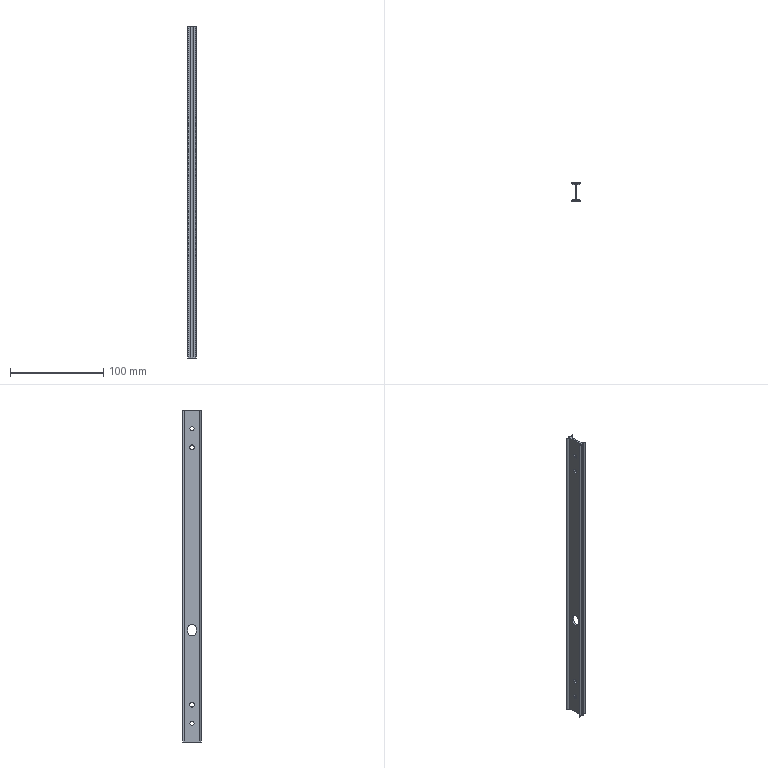Part | SolidWorks | features BaseBody 1, RefAxis 1 | 1 solid | 47 faces | box 9.344 x 19.967 x 355.6 mm | volume 18790 mm3 | cylinder 29 | plane 18 | commonest cylinder face diameters 4.5 x10 3.7 x8 1 x4 2 x4 9.5 x3
STEP:
#1=CARTESIAN_POINT('',(7.5,11.15,17.75));
#2=VERTEX_POINT('',#1);
#3=CARTESIAN_POINT('',(7.5,11.15,22.25));
#4=VERTEX_POINT('',#3);
#5=CARTESIAN_POINT('',(7.5,11.15,20.));
#6=DIRECTION('',(-1.,0.,0.));
#7=DIRECTION('',(0.,0.,1.));
#8=AXIS2_PLACEMENT_3D('',#5,#6,#7);
#9=CIRCLE('',#8,2.25);
#10=EDGE_CURVE('',#2,#4,#9,.T.);
#11=ORIENTED_EDGE('',*,*,#10,.F.);
#12=CARTESIAN_POINT('',(5.5,11.15,17.75));
#13=VERTEX_POINT('',#12);
#14=CARTESIAN_POINT('',(0.,11.15,17.75));
#15=DIRECTION('',(-1.,0.,0.));
#16=VECTOR('',#15,1000.);
#17=LINE('',#14,#16);
#18=EDGE_CURVE('',#2,#13,#17,.T.);
#19=ORIENTED_EDGE('',*,*,#18,.T.);
#20=CARTESIAN_POINT('',(5.5,11.15,22.25));
#21=VERTEX_POINT('',#20);
#22=CARTESIAN_POINT('',(5.5,11.15,20.));
#23=DIRECTION('',(1.,0.,0.));
#24=DIRECTION('',(0.,0.,1.));
#25=AXIS2_PLACEMENT_3D('',#22,#23,#24);
#26=CIRCLE('',#25,2.25);
#27=EDGE_CURVE('',#21,#13,#26,.T.);
#28=ORIENTED_EDGE('',*,*,#27,.F.);
#29=CARTESIAN_POINT('',(0.,11.15,22.25));
#30=DIRECTION('',(-1.,0.,0.));
#31=VECTOR('',#30,1000.);
#32=LINE('',#29,#31);
#33=EDGE_CURVE('',#4,#21,#32,.T.);
#34=ORIENTED_EDGE('',*,*,#33,.F.);
#35=EDGE_LOOP('',(#11,#19,#28,#34));
#36=FACE_OUTER_BOUND('',#35,.T.);
#37=CARTESIAN_POINT('',(0.,11.15,20.));
#38=DIRECTION('',(-1.,0.,0.));
#39=DIRECTION('',(0.,0.,1.));
#40=AXIS2_PLACEMENT_3D('',#37,#38,#39);
#41=CYLINDRICAL_SURFACE('',#40,2.25);
#42=ADVANCED_FACE('',(#36),#41,.F.);
#43=CARTESIAN_POINT('',(7.5,11.15,333.35));
#44=VERTEX_POINT('',#43);
#45=CARTESIAN_POINT('',(7.5,11.15,337.85));
#46=VERTEX_POINT('',#45);
#47=CARTESIAN_POINT('',(7.5,11.15,335.6));
#48=DIRECTION('',(-1.,0.,0.));
#49=DIRECTION('',(0.,0.,1.));
#50=AXIS2_PLACEMENT_3D('',#47,#48,#49);
#51=CIRCLE('',#50,2.25);
#52=EDGE_CURVE('',#44,#46,#51,.T.);
#53=ORIENTED_EDGE('',*,*,#52,.F.);
#54=CARTESIAN_POINT('',(5.5,11.15,333.35));
#55=VERTEX_POINT('',#54);
#56=CARTESIAN_POINT('',(0.,11.15,333.35));
#57=DIRECTION('',(-1.,0.,0.));
#58=VECTOR('',#57,1000.);
#59=LINE('',#56,#58);
#60=EDGE_CURVE('',#44,#55,#59,.T.);
#61=ORIENTED_EDGE('',*,*,#60,.T.);
#62=CARTESIAN_POINT('',(5.5,11.15,337.85));
#63=VERTEX_POINT('',#62);
#64=CARTESIAN_POINT('',(5.5,11.15,335.6));
#65=DIRECTION('',(1.,0.,0.));
#66=DIRECTION('',(0.,0.,1.));
#67=AXIS2_PLACEMENT_3D('',#64,#65,#66);
#68=CIRCLE('',#67,2.25);
#69=EDGE_CURVE('',#63,#55,#68,.T.);
#70=ORIENTED_EDGE('',*,*,#69,.F.);
#71=CARTESIAN_POINT('',(0.,11.15,337.85));
#72=DIRECTION('',(-1.,0.,0.));
#73=VECTOR('',#72,1000.);
#74=LINE('',#71,#73);
#75=EDGE_CURVE('',#46,#63,#74,.T.);
#76=ORIENTED_EDGE('',*,*,#75,.F.);
#77=EDGE_LOOP('',(#53,#61,#70,#76));
#78=FACE_OUTER_BOUND('',#77,.T.);
#79=CARTESIAN_POINT('',(0.,11.15,335.6));
#80=DIRECTION('',(-1.,0.,0.));
#81=DIRECTION('',(0.,0.,1.));
#82=AXIS2_PLACEMENT_3D('',#79,#80,#81);
#83=CYLINDRICAL_SURFACE('',#82,2.25);
#84=ADVANCED_FACE('',(#78),#83,.F.);
#85=CARTESIAN_POINT('',(7.5,11.15,318.25));
#86=VERTEX_POINT('',#85);
#87=CARTESIAN_POINT('',(7.5,13.4,316.));
#88=VERTEX_POINT('',#87);
#89=CARTESIAN_POINT('',(7.5,11.15,316.));
#90=DIRECTION('',(-1.,0.,0.));
#91=DIRECTION('',(0.,0.,1.));
#92=AXIS2_PLACEMENT_3D('',#89,#90,#91);
#93=CIRCLE('',#92,2.25);
#94=EDGE_CURVE('',#86,#88,#93,.T.);
#95=ORIENTED_EDGE('',*,*,#94,.F.);
#96=CARTESIAN_POINT('',(5.5,11.15,318.25));
#97=VERTEX_POINT('',#96);
#98=CARTESIAN_POINT('',(0.,11.15,318.25));
#99=DIRECTION('',(-1.,0.,0.));
#100=VECTOR('',#99,1000.);
#101=LINE('',#98,#100);
#102=EDGE_CURVE('',#86,#97,#101,.T.);
#103=ORIENTED_EDGE('',*,*,#102,.T.);
#104=CARTESIAN_POINT('',(5.5,13.4,316.));
#105=VERTEX_POINT('',#104);
#106=CARTESIAN_POINT('',(5.5,11.15,316.));
#107=DIRECTION('',(1.,0.,0.));
#108=DIRECTION('',(0.,0.,1.));
#109=AXIS2_PLACEMENT_3D('',#106,#107,#108);
#110=CIRCLE('',#109,2.25);
#111=EDGE_CURVE('',#105,#97,#110,.T.);
#112=ORIENTED_EDGE('',*,*,#111,.F.);
#113=CARTESIAN_POINT('',(0.,13.4,316.));
#114=DIRECTION('',(-1.,0.,0.));
#115=VECTOR('',#114,1000.);
#116=LINE('',#113,#115);
#117=EDGE_CURVE('',#88,#105,#116,.T.);
#118=ORIENTED_EDGE('',*,*,#117,.F.);
#119=EDGE_LOOP('',(#95,#103,#112,#118));
#120=FACE_OUTER_BOUND('',#119,.T.);
#121=CARTESIAN_POINT('',(0.,11.15,316.));
#122=DIRECTION('',(-1.,0.,0.));
#123=DIRECTION('',(0.,0.,1.));
#124=AXIS2_PLACEMENT_3D('',#121,#122,#123);
#125=CYLINDRICAL_SURFACE('',#124,2.25);
#126=ADVANCED_FACE('',(#120),#125,.F.);
#127=CARTESIAN_POINT('',(7.5,11.15,42.65));
#128=VERTEX_POINT('',#127);
#129=CARTESIAN_POINT('',(7.5,13.4,40.4));
#130=VERTEX_POINT('',#129);
#131=CARTESIAN_POINT('',(7.5,11.15,40.4));
#132=DIRECTION('',(-1.,0.,0.));
#133=DIRECTION('',(0.,0.,1.));
#134=AXIS2_PLACEMENT_3D('',#131,#132,#133);
#135=CIRCLE('',#134,2.25);
#136=EDGE_CURVE('',#128,#130,#135,.T.);
#137=ORIENTED_EDGE('',*,*,#136,.F.);
#138=CARTESIAN_POINT('',(5.5,11.15,42.65));
#139=VERTEX_POINT('',#138);
#140=CARTESIAN_POINT('',(0.,11.15,42.65));
#141=DIRECTION('',(-1.,0.,0.));
#142=VECTOR('',#141,1000.);
#143=LINE('',#140,#142);
#144=EDGE_CURVE('',#128,#139,#143,.T.);
#145=ORIENTED_EDGE('',*,*,#144,.T.);
#146=CARTESIAN_POINT('',(5.5,13.4,40.4));
#147=VERTEX_POINT('',#146);
#148=CARTESIAN_POINT('',(5.5,11.15,40.4));
#149=DIRECTION('',(1.,0.,0.));
#150=DIRECTION('',(0.,0.,1.));
#151=AXIS2_PLACEMENT_3D('',#148,#149,#150);
#152=CIRCLE('',#151,2.25);
#153=EDGE_CURVE('',#147,#139,#152,.T.);
#154=ORIENTED_EDGE('',*,*,#153,.F.);
#155=CARTESIAN_POINT('',(0.,13.4,40.4));
#156=DIRECTION('',(-1.,0.,0.));
#157=VECTOR('',#156,1000.);
#158=LINE('',#155,#157);
#159=EDGE_CURVE('',#130,#147,#158,.T.);
#160=ORIENTED_EDGE('',*,*,#159,.F.);
#161=EDGE_LOOP('',(#137,#145,#154,#160));
#162=FACE_OUTER_BOUND('',#161,.T.);
#163=CARTESIAN_POINT('',(0.,11.15,40.4));
#164=DIRECTION('',(-1.,0.,0.));
#165=DIRECTION('',(0.,0.,1.));
#166=AXIS2_PLACEMENT_3D('',#163,#164,#165);
#167=CYLINDRICAL_SURFACE('',#166,2.25);
#168=ADVANCED_FACE('',(#162),#167,.F.);
#169=CARTESIAN_POINT('',(7.5,11.15,126.25));
#170=VERTEX_POINT('',#169);
#171=CARTESIAN_POINT('',(7.5,15.9,121.5));
#172=VERTEX_POINT('',#171);
#173=CARTESIAN_POINT('',(7.5,11.15,121.5));
#174=DIRECTION('',(-1.,0.,0.));
#175=DIRECTION('',(0.,0.,1.));
#176=AXIS2_PLACEMENT_3D('',#173,#174,#175);
#177=CIRCLE('',#176,4.75);
#178=EDGE_CURVE('',#170,#172,#177,.T.);
#179=ORIENTED_EDGE('',*,*,#178,.F.);
#180=CARTESIAN_POINT('',(5.5,11.15,126.25));
#181=VERTEX_POINT('',#180);
#182=CARTESIAN_POINT('',(0.,11.15,126.25));
#183=DIRECTION('',(-1.,0.,0.));
#184=VECTOR('',#183,1000.);
#185=LINE('',#182,#184);
#186=EDGE_CURVE('',#170,#181,#185,.T.);
#187=ORIENTED_EDGE('',*,*,#186,.T.);
#188=CARTESIAN_POINT('',(5.5,15.9,121.5));
#189=VERTEX_POINT('',#188);
#190=CARTESIAN_POINT('',(5.5,11.15,121.5));
#191=DIRECTION('',(1.,0.,0.));
#192=DIRECTION('',(0.,0.,1.));
#193=AXIS2_PLACEMENT_3D('',#190,#191,#192);
#194=CIRCLE('',#193,4.75);
#195=EDGE_CURVE('',#189,#181,#194,.T.);
#196=ORIENTED_EDGE('',*,*,#195,.F.);
#197=CARTESIAN_POINT('',(0.,15.9,121.5));
#198=DIRECTION('',(1.,0.,0.));
#199=VECTOR('',#198,1000.);
#200=LINE('',#197,#199);
#201=EDGE_CURVE('',#189,#172,#200,.T.);
#202=ORIENTED_EDGE('',*,*,#201,.T.);
#203=EDGE_LOOP('',(#179,#187,#196,#202));
#204=FACE_OUTER_BOUND('',#203,.T.);
#205=CARTESIAN_POINT('',(0.,11.15,121.5));
#206=DIRECTION('',(-1.,0.,0.));
#207=DIRECTION('',(0.,0.,1.));
#208=AXIS2_PLACEMENT_3D('',#205,#206,#207);
#209=CYLINDRICAL_SURFACE('',#208,4.75);
#210=ADVANCED_FACE('',(#204),#209,.F.);
#211=CARTESIAN_POINT('',(5.5,19.376,0.));
#212=VERTEX_POINT('',#211);
#213=CARTESIAN_POINT('',(5.5,2.924,0.));
#214=VERTEX_POINT('',#213);
#215=CARTESIAN_POINT('',(5.5,2.924,0.));
#216=DIRECTION('',(0.,-1.,0.));
#217=VECTOR('',#216,1000.);
#218=LINE('',#215,#217);
#219=EDGE_CURVE('',#212,#214,#218,.T.);
#220=ORIENTED_EDGE('',*,*,#219,.T.);
#221=CARTESIAN_POINT('',(5.5,2.924,355.6));
#222=VERTEX_POINT('',#221);
#223=CARTESIAN_POINT('',(5.5,2.924,0.));
#224=DIRECTION('',(0.,0.,1.));
#225=VECTOR('',#224,1000.);
#226=LINE('',#223,#225);
#227=EDGE_CURVE('',#214,#222,#226,.T.);
#228=ORIENTED_EDGE('',*,*,#227,.T.);
#229=CARTESIAN_POINT('',(5.5,19.376,355.6));
#230=VERTEX_POINT('',#229);
#231=CARTESIAN_POINT('',(5.5,2.924,355.6));
#232=DIRECTION('',(0.,1.,0.));
#233=VECTOR('',#232,1000.);
#234=LINE('',#231,#233);
#235=EDGE_CURVE('',#222,#230,#234,.T.);
#236=ORIENTED_EDGE('',*,*,#235,.T.);
#237=CARTESIAN_POINT('',(5.5,19.376,0.));
#238=DIRECTION('',(0.,0.,-1.));
#239=VECTOR('',#238,1000.);
#240=LINE('',#237,#239);
#241=EDGE_CURVE('',#230,#212,#240,.T.);
#242=ORIENTED_EDGE('',*,*,#241,.T.);
#243=EDGE_LOOP('',(#220,#228,#236,#242));
#244=FACE_OUTER_BOUND('',#243,.T.);
#245=ORIENTED_EDGE('',*,*,#27,.T.);
#246=CARTESIAN_POINT('',(5.5,11.15,20.));
#247=DIRECTION('',(1.,0.,0.));
#248=DIRECTION('',(0.,0.,1.));
#249=AXIS2_PLACEMENT_3D('',#246,#247,#248);
#250=CIRCLE('',#249,2.25);
#251=EDGE_CURVE('',#13,#21,#250,.T.);
#252=ORIENTED_EDGE('',*,*,#251,.T.);
#253=EDGE_LOOP('',(#245,#252));
#254=FACE_BOUND('',#253,.T.);
#255=ORIENTED_EDGE('',*,*,#69,.T.);
#256=CARTESIAN_POINT('',(5.5,11.15,335.6));
#257=DIRECTION('',(1.,0.,0.));
#258=DIRECTION('',(0.,0.,1.));
#259=AXIS2_PLACEMENT_3D('',#256,#257,#258);
#260=CIRCLE('',#259,2.25);
#261=EDGE_CURVE('',#55,#63,#260,.T.);
#262=ORIENTED_EDGE('',*,*,#261,.T.);
#263=EDGE_LOOP('',(#255,#262));
#264=FACE_BOUND('',#263,.T.);
#265=CARTESIAN_POINT('',(5.5,8.9,315.2));
#266=VERTEX_POINT('',#265);
#267=CARTESIAN_POINT('',(5.5,13.4,315.2));
#268=VERTEX_POINT('',#267);
#269=CARTESIAN_POINT('',(5.5,11.15,315.2));
#270=DIRECTION('',(1.,0.,0.));
#271=DIRECTION('',(0.,0.,1.));
#272=AXIS2_PLACEMENT_3D('',#269,#270,#271);
#273=CIRCLE('',#272,2.25);
#274=EDGE_CURVE('',#266,#268,#273,.T.);
#275=ORIENTED_EDGE('',*,*,#274,.T.);
#276=CARTESIAN_POINT('',(5.5,13.4,316.));
#277=DIRECTION('',(0.,0.,1.));
#278=VECTOR('',#277,1000.);
#279=LINE('',#276,#278);
#280=EDGE_CURVE('',#268,#105,#279,.T.);
#281=ORIENTED_EDGE('',*,*,#280,.T.);
#282=ORIENTED_EDGE('',*,*,#111,.T.);
#283=CARTESIAN_POINT('',(5.5,8.9,316.));
#284=VERTEX_POINT('',#283);
#285=CARTESIAN_POINT('',(5.5,11.15,316.));
#286=DIRECTION('',(1.,0.,0.));
#287=DIRECTION('',(0.,0.,1.));
#288=AXIS2_PLACEMENT_3D('',#285,#286,#287);
#289=CIRCLE('',#288,2.25);
#290=EDGE_CURVE('',#97,#284,#289,.T.);
#291=ORIENTED_EDGE('',*,*,#290,.T.);
#292=CARTESIAN_POINT('',(5.5,8.9,315.2));
#293=DIRECTION('',(0.,0.,-1.));
#294=VECTOR('',#293,1000.);
#295=LINE('',#292,#294);
#296=EDGE_CURVE('',#284,#266,#295,.T.);
#297=ORIENTED_EDGE('',*,*,#296,.T.);
#298=EDGE_LOOP('',(#275,#281,#282,#291,#297));
#299=FACE_BOUND('',#298,.T.);
#300=CARTESIAN_POINT('',(5.5,8.9,39.6));
#301=VERTEX_POINT('',#300);
#302=CARTESIAN_POINT('',(5.5,13.4,39.6));
#303=VERTEX_POINT('',#302);
#304=CARTESIAN_POINT('',(5.5,11.15,39.6));
#305=DIRECTION('',(1.,0.,0.));
#306=DIRECTION('',(0.,0.,1.));
#307=AXIS2_PLACEMENT_3D('',#304,#305,#306);
#308=CIRCLE('',#307,2.25);
#309=EDGE_CURVE('',#301,#303,#308,.T.);
#310=ORIENTED_EDGE('',*,*,#309,.T.);
#311=CARTESIAN_POINT('',(5.5,13.4,40.4));
#312=DIRECTION('',(0.,0.,1.));
#313=VECTOR('',#312,1000.);
#314=LINE('',#311,#313);
#315=EDGE_CURVE('',#303,#147,#314,.T.);
#316=ORIENTED_EDGE('',*,*,#315,.T.);
#317=ORIENTED_EDGE('',*,*,#153,.T.);
#318=CARTESIAN_POINT('',(5.5,8.9,40.4));
#319=VERTEX_POINT('',#318);
#320=CARTESIAN_POINT('',(5.5,11.15,40.4));
#321=DIRECTION('',(1.,0.,0.));
#322=DIRECTION('',(0.,0.,1.));
#323=AXIS2_PLACEMENT_3D('',#320,#321,#322);
#324=CIRCLE('',#323,2.25);
#325=EDGE_CURVE('',#139,#319,#324,.T.);
#326=ORIENTED_EDGE('',*,*,#325,.T.);
#327=CARTESIAN_POINT('',(5.5,8.9,39.6));
#328=DIRECTION('',(0.,0.,-1.));
#329=VECTOR('',#328,1000.);
#330=LINE('',#327,#329);
#331=EDGE_CURVE('',#319,#301,#330,.T.);
#332=ORIENTED_EDGE('',*,*,#331,.T.);
#333=EDGE_LOOP('',(#310,#316,#317,#326,#332));
#334=FACE_BOUND('',#333,.T.);
#335=CARTESIAN_POINT('',(5.5,6.4,118.5));
#336=VERTEX_POINT('',#335);
#337=CARTESIAN_POINT('',(5.5,15.9,118.5));
#338=VERTEX_POINT('',#337);
#339=CARTESIAN_POINT('',(5.5,11.15,118.5));
#340=DIRECTION('',(1.,0.,0.));
#341=DIRECTION('',(0.,0.,1.));
#342=AXIS2_PLACEMENT_3D('',#339,#340,#341);
#343=CIRCLE('',#342,4.75);
#344=EDGE_CURVE('',#336,#338,#343,.T.);
#345=ORIENTED_EDGE('',*,*,#344,.T.);
#346=CARTESIAN_POINT('',(5.5,15.9,0.));
#347=DIRECTION('',(0.,0.,1.));
#348=VECTOR('',#347,1000.);
#349=LINE('',#346,#348);
#350=EDGE_CURVE('',#338,#189,#349,.T.);
#351=ORIENTED_EDGE('',*,*,#350,.T.);
#352=ORIENTED_EDGE('',*,*,#195,.T.);
#353=CARTESIAN_POINT('',(5.5,6.4,121.5));
#354=VERTEX_POINT('',#353);
#355=CARTESIAN_POINT('',(5.5,11.15,121.5));
#356=DIRECTION('',(1.,0.,0.));
#357=DIRECTION('',(0.,0.,1.));
#358=AXIS2_PLACEMENT_3D('',#355,#356,#357);
#359=CIRCLE('',#358,4.75);
#360=EDGE_CURVE('',#181,#354,#359,.T.);
#361=ORIENTED_EDGE('',*,*,#360,.T.);
#362=CARTESIAN_POINT('',(5.5,6.4,0.));
#363=DIRECTION('',(0.,0.,-1.));
#364=VECTOR('',#363,1000.);
#365=LINE('',#362,#364);
#366=EDGE_CURVE('',#354,#336,#365,.T.);
#367=ORIENTED_EDGE('',*,*,#366,.T.);
#368=EDGE_LOOP('',(#345,#351,#352,#361,#367));
#369=FACE_BOUND('',#368,.T.);
#370=CARTESIAN_POINT('',(5.5,2.924,0.));
#371=DIRECTION('',(-1.,0.,0.));
#372=DIRECTION('',(0.,0.,1.));
#373=AXIS2_PLACEMENT_3D('',#370,#371,#372);
#374=PLANE('',#373);
#375=ADVANCED_FACE('',(#244,#254,#264,#299,#334,#369),#374,.T.);
#376=ORIENTED_EDGE('',*,*,#227,.F.);
#377=CARTESIAN_POINT('',(4.713,2.514,0.));
#378=VERTEX_POINT('',#377);
#379=CARTESIAN_POINT('',(5.,2.924,0.));
#380=DIRECTION('',(0.,0.,1.));
#381=DIRECTION('',(-1.,0.,0.));
#382=AXIS2_PLACEMENT_3D('',#379,#380,#381);
#383=CIRCLE('',#382,0.5);
#384=EDGE_CURVE('',#378,#214,#383,.T.);
#385=ORIENTED_EDGE('',*,*,#384,.F.);
#386=CARTESIAN_POINT('',(4.713,2.514,355.6));
#387=VERTEX_POINT('',#386);
#388=CARTESIAN_POINT('',(4.713,2.514,0.));
#389=DIRECTION('',(0.,0.,-1.));
#390=VECTOR('',#389,1000.);
#391=LINE('',#388,#390);
#392=EDGE_CURVE('',#387,#378,#391,.T.);
#393=ORIENTED_EDGE('',*,*,#392,.F.);
#394=CARTESIAN_POINT('',(5.,2.924,355.6));
#395=DIRECTION('',(0.,0.,-1.));
#396=DIRECTION('',(-1.,0.,0.));
#397=AXIS2_PLACEMENT_3D('',#394,#395,#396);
#398=CIRCLE('',#397,0.5);
#399=EDGE_CURVE('',#222,#387,#398,.T.);
#400=ORIENTED_EDGE('',*,*,#399,.F.);
#401=EDGE_LOOP('',(#376,#385,#393,#400));
#402=FACE_OUTER_BOUND('',#401,.T.);
#403=CARTESIAN_POINT('',(5.,2.924,0.));
#404=DIRECTION('',(0.,0.,-1.));
#405=DIRECTION('',(-1.,0.,0.));
#406=AXIS2_PLACEMENT_3D('',#403,#404,#405);
#407=CYLINDRICAL_SURFACE('',#406,0.5);
#408=ADVANCED_FACE('',(#402),#407,.F.);
#409=CARTESIAN_POINT('',(2.279,21.058,0.));
#410=VERTEX_POINT('',#409);
#411=CARTESIAN_POINT('',(1.828,20.979,0.));
#412=VERTEX_POINT('',#411);
#413=CARTESIAN_POINT('',(1.828,20.979,0.));
#414=DIRECTION('',(-0.9848,-0.1736,0.));
#415=VECTOR('',#414,1000.);
#416=LINE('',#413,#415);
#417=EDGE_CURVE('',#410,#412,#416,.T.);
#418=ORIENTED_EDGE('',*,*,#417,.F.);
#419=CARTESIAN_POINT('',(4.852,20.894,0.));
#420=VERTEX_POINT('',#419);
#421=CARTESIAN_POINT('',(3.65,22.3,0.));
#422=DIRECTION('',(0.,0.,-1.));
#423=DIRECTION('',(-1.,0.,0.));
#424=AXIS2_PLACEMENT_3D('',#421,#422,#423);
#425=CIRCLE('',#424,1.85);
#426=EDGE_CURVE('',#420,#410,#425,.T.);
#427=ORIENTED_EDGE('',*,*,#426,.F.);
#428=CARTESIAN_POINT('',(6.321,20.706,0.));
#429=VERTEX_POINT('',#428);
#430=CARTESIAN_POINT('',(5.501,20.133,0.));
#431=DIRECTION('',(0.,0.,1.));
#432=DIRECTION('',(-1.,0.,0.));
#433=AXIS2_PLACEMENT_3D('',#430,#431,#432);
#434=CIRCLE('',#433,1.);
#435=EDGE_CURVE('',#429,#420,#434,.T.);
#436=ORIENTED_EDGE('',*,*,#435,.F.);
#437=CARTESIAN_POINT('',(6.5,20.45,0.));
#438=VERTEX_POINT('',#437);
#439=CARTESIAN_POINT('',(6.321,20.706,0.));
#440=DIRECTION('',(-0.5725,0.8199,0.));
#441=VECTOR('',#440,1000.);
#442=LINE('',#439,#441);
#443=EDGE_CURVE('',#438,#429,#442,.T.);
#444=ORIENTED_EDGE('',*,*,#443,.F.);
#445=CARTESIAN_POINT('',(6.679,20.706,0.));
#446=VERTEX_POINT('',#445);
#447=CARTESIAN_POINT('',(6.5,20.45,0.));
#448=DIRECTION('',(-0.5725,-0.8199,0.));
#449=VECTOR('',#448,1000.);
#450=LINE('',#447,#449);
#451=EDGE_CURVE('',#446,#438,#450,.T.);
#452=ORIENTED_EDGE('',*,*,#451,.F.);
#453=CARTESIAN_POINT('',(8.148,20.894,0.));
#454=VERTEX_POINT('',#453);
#455=CARTESIAN_POINT('',(7.499,20.133,0.));
#456=DIRECTION('',(0.,0.,1.));
#457=DIRECTION('',(-1.,0.,0.));
#458=AXIS2_PLACEMENT_3D('',#455,#456,#457);
#459=CIRCLE('',#458,1.);
#460=EDGE_CURVE('',#454,#446,#459,.T.);
#461=ORIENTED_EDGE('',*,*,#460,.F.);
#462=CARTESIAN_POINT('',(10.721,21.058,0.));
#463=VERTEX_POINT('',#462);
#464=CARTESIAN_POINT('',(9.35,22.3,0.));
#465=DIRECTION('',(0.,0.,-1.));
#466=DIRECTION('',(-1.,0.,0.));
#467=AXIS2_PLACEMENT_3D('',#464,#465,#466);
#468=CIRCLE('',#467,1.85);
#469=EDGE_CURVE('',#463,#454,#468,.T.);
#470=ORIENTED_EDGE('',*,*,#469,.F.);
#471=CARTESIAN_POINT('',(11.172,20.979,0.));
#472=VERTEX_POINT('',#471);
#473=CARTESIAN_POINT('',(10.721,21.058,0.));
#474=DIRECTION('',(-0.9848,0.1736,0.));
#475=VECTOR('',#474,1000.);
#476=LINE('',#473,#475);
#477=EDGE_CURVE('',#472,#463,#476,.T.);
#478=ORIENTED_EDGE('',*,*,#477,.F.);
#479=CARTESIAN_POINT('',(8.287,19.786,0.));
#480=VERTEX_POINT('',#479);
#481=CARTESIAN_POINT('',(9.35,21.3,0.));
#482=DIRECTION('',(0.,0.,1.));
#483=DIRECTION('',(-1.,0.,0.));
#484=AXIS2_PLACEMENT_3D('',#481,#482,#483);
#485=CIRCLE('',#484,1.85);
#486=EDGE_CURVE('',#480,#472,#485,.T.);
#487=ORIENTED_EDGE('',*,*,#486,.F.);
#488=CARTESIAN_POINT('',(7.5,19.376,0.));
#489=VERTEX_POINT('',#488);
#490=CARTESIAN_POINT('',(8.,19.376,0.));
#491=DIRECTION('',(0.,0.,1.));
#492=DIRECTION('',(-1.,0.,0.));
#493=AXIS2_PLACEMENT_3D('',#490,#491,#492);
#494=CIRCLE('',#493,0.5);
#495=EDGE_CURVE('',#480,#489,#494,.T.);
#496=ORIENTED_EDGE('',*,*,#495,.T.);
#497=CARTESIAN_POINT('',(7.5,2.924,0.));
#498=VERTEX_POINT('',#497);
#499=CARTESIAN_POINT('',(7.5,0.,0.));
#500=DIRECTION('',(0.,1.,0.));
#501=VECTOR('',#500,1000.);
#502=LINE('',#499,#501);
#503=EDGE_CURVE('',#498,#489,#502,.T.);
#504=ORIENTED_EDGE('',*,*,#503,.F.);
#505=CARTESIAN_POINT('',(8.287,2.514,0.));
#506=VERTEX_POINT('',#505);
#507=CARTESIAN_POINT('',(8.,2.924,0.));
#508=DIRECTION('',(0.,0.,1.));
#509=DIRECTION('',(-1.,0.,0.));
#510=AXIS2_PLACEMENT_3D('',#507,#508,#509);
#511=CIRCLE('',#510,0.5);
#512=EDGE_CURVE('',#498,#506,#511,.T.);
#513=ORIENTED_EDGE('',*,*,#512,.T.);
#514=CARTESIAN_POINT('',(11.172,1.321,0.));
#515=VERTEX_POINT('',#514);
#516=CARTESIAN_POINT('',(9.35,1.,0.));
#517=DIRECTION('',(0.,0.,1.));
#518=DIRECTION('',(-1.,0.,0.));
#519=AXIS2_PLACEMENT_3D('',#516,#517,#518);
#520=CIRCLE('',#519,1.85);
#521=EDGE_CURVE('',#515,#506,#520,.T.);
#522=ORIENTED_EDGE('',*,*,#521,.F.);
#523=CARTESIAN_POINT('',(10.721,1.242,0.));
#524=VERTEX_POINT('',#523);
#525=CARTESIAN_POINT('',(11.172,1.321,0.));
#526=DIRECTION('',(0.9848,0.1736,0.));
#527=VECTOR('',#526,1000.);
#528=LINE('',#525,#527);
#529=EDGE_CURVE('',#524,#515,#528,.T.);
#530=ORIENTED_EDGE('',*,*,#529,.F.);
#531=CARTESIAN_POINT('',(8.148,1.406,0.));
#532=VERTEX_POINT('',#531);
#533=CARTESIAN_POINT('',(9.35,0.,0.));
#534=DIRECTION('',(0.,0.,-1.));
#535=DIRECTION('',(-1.,0.,0.));
#536=AXIS2_PLACEMENT_3D('',#533,#534,#535);
#537=CIRCLE('',#536,1.85);
#538=EDGE_CURVE('',#532,#524,#537,.T.);
#539=ORIENTED_EDGE('',*,*,#538,.F.);
#540=CARTESIAN_POINT('',(6.679,1.594,0.));
#541=VERTEX_POINT('',#540);
#542=CARTESIAN_POINT('',(7.499,2.167,0.));
#543=DIRECTION('',(0.,0.,1.));
#544=DIRECTION('',(-1.,0.,0.));
#545=AXIS2_PLACEMENT_3D('',#542,#543,#544);
#546=CIRCLE('',#545,1.);
#547=EDGE_CURVE('',#541,#532,#546,.T.);
#548=ORIENTED_EDGE('',*,*,#547,.F.);
#549=CARTESIAN_POINT('',(6.5,1.85,0.));
#550=VERTEX_POINT('',#549);
#551=CARTESIAN_POINT('',(6.679,1.594,0.));
#552=DIRECTION('',(0.5725,-0.8199,0.));
#553=VECTOR('',#552,1000.);
#554=LINE('',#551,#553);
#555=EDGE_CURVE('',#550,#541,#554,.T.);
#556=ORIENTED_EDGE('',*,*,#555,.F.);
#557=CARTESIAN_POINT('',(6.321,1.594,0.));
#558=VERTEX_POINT('',#557);
#559=CARTESIAN_POINT('',(6.5,1.85,0.));
#560=DIRECTION('',(0.5725,0.8199,0.));
#561=VECTOR('',#560,1000.);
#562=LINE('',#559,#561);
#563=EDGE_CURVE('',#558,#550,#562,.T.);
#564=ORIENTED_EDGE('',*,*,#563,.F.);
#565=CARTESIAN_POINT('',(4.852,1.406,0.));
#566=VERTEX_POINT('',#565);
#567=CARTESIAN_POINT('',(5.501,2.167,0.));
#568=DIRECTION('',(0.,0.,1.));
#569=DIRECTION('',(-1.,0.,0.));
#570=AXIS2_PLACEMENT_3D('',#567,#568,#569);
#571=CIRCLE('',#570,1.);
#572=EDGE_CURVE('',#566,#558,#571,.T.);
#573=ORIENTED_EDGE('',*,*,#572,.F.);
#574=CARTESIAN_POINT('',(2.279,1.242,0.));
#575=VERTEX_POINT('',#574);
#576=CARTESIAN_POINT('',(3.65,0.,0.));
#577=DIRECTION('',(0.,0.,-1.));
#578=DIRECTION('',(-1.,0.,0.));
#579=AXIS2_PLACEMENT_3D('',#576,#577,#578);
#580=CIRCLE('',#579,1.85);
#581=EDGE_CURVE('',#575,#566,#580,.T.);
#582=ORIENTED_EDGE('',*,*,#581,.F.);
#583=CARTESIAN_POINT('',(1.828,1.321,0.));
#584=VERTEX_POINT('',#583);
#585=CARTESIAN_POINT('',(2.279,1.242,0.));
#586=DIRECTION('',(0.9848,-0.1736,0.));
#587=VECTOR('',#586,1000.);
#588=LINE('',#585,#587);
#589=EDGE_CURVE('',#584,#575,#588,.T.);
#590=ORIENTED_EDGE('',*,*,#589,.F.);
#591=CARTESIAN_POINT('',(3.65,1.,0.));
#592=DIRECTION('',(0.,0.,1.));
#593=DIRECTION('',(-1.,0.,0.));
#594=AXIS2_PLACEMENT_3D('',#591,#592,#593);
#595=CIRCLE('',#594,1.85);
#596=EDGE_CURVE('',#378,#584,#595,.T.);
#597=ORIENTED_EDGE('',*,*,#596,.F.);
#598=ORIENTED_EDGE('',*,*,#384,.T.);
#599=ORIENTED_EDGE('',*,*,#219,.F.);
#600=CARTESIAN_POINT('',(4.713,19.786,0.));
#601=VERTEX_POINT('',#600);
#602=CARTESIAN_POINT('',(5.,19.376,0.));
#603=DIRECTION('',(0.,0.,-1.));
#604=DIRECTION('',(-1.,0.,0.));
#605=AXIS2_PLACEMENT_3D('',#602,#603,#604);
#606=CIRCLE('',#605,0.5);
#607=EDGE_CURVE('',#601,#212,#606,.T.);
#608=ORIENTED_EDGE('',*,*,#607,.F.);
#609=CARTESIAN_POINT('',(3.65,21.3,0.));
#610=DIRECTION('',(0.,0.,1.));
#611=DIRECTION('',(-1.,0.,0.));
#612=AXIS2_PLACEMENT_3D('',#609,#610,#611);
#613=CIRCLE('',#612,1.85);
#614=EDGE_CURVE('',#412,#601,#613,.T.);
#615=ORIENTED_EDGE('',*,*,#614,.F.);
#616=EDGE_LOOP('',(#418,#427,#436,#444,#452,#461,#470,#478,#487,#496,#504,#513,#522,#530,#539,#548,#556,#564,#573,#582,#590,#597,#598,#599,#608,#615));
#617=FACE_OUTER_BOUND('',#616,.T.);
#618=CARTESIAN_POINT('',(0.,0.,0.));
#619=DIRECTION('',(0.,0.,1.));
#620=DIRECTION('',(1.,0.,0.));
#621=AXIS2_PLACEMENT_3D('',#618,#619,#620);
#622=PLANE('',#621);
#623=ADVANCED_FACE('',(#617),#622,.F.);
#624=CARTESIAN_POINT('',(4.713,19.786,355.6));
#625=VERTEX_POINT('',#624);
#626=CARTESIAN_POINT('',(4.713,19.786,0.));
#627=DIRECTION('',(0.,0.,1.));
#628=VECTOR('',#627,1000.);
#629=LINE('',#626,#628);
#630=EDGE_CURVE('',#601,#625,#629,.T.);
#631=ORIENTED_EDGE('',*,*,#630,.F.);
#632=ORIENTED_EDGE('',*,*,#607,.T.);
#633=ORIENTED_EDGE('',*,*,#241,.F.);
#634=CARTESIAN_POINT('',(5.,19.376,355.6));
#635=DIRECTION('',(0.,0.,-1.));
#636=DIRECTION('',(-1.,0.,0.));
#637=AXIS2_PLACEMENT_3D('',#634,#635,#636);
#638=CIRCLE('',#637,0.5);
#639=EDGE_CURVE('',#625,#230,#638,.T.);
#640=ORIENTED_EDGE('',*,*,#639,.F.);
#641=EDGE_LOOP('',(#631,#632,#633,#640));
#642=FACE_OUTER_BOUND('',#641,.T.);
#643=CARTESIAN_POINT('',(5.,19.376,0.));
#644=DIRECTION('',(0.,0.,-1.));
#645=DIRECTION('',(-1.,0.,0.));
#646=AXIS2_PLACEMENT_3D('',#643,#644,#645);
#647=CYLINDRICAL_SURFACE('',#646,0.5);
#648=ADVANCED_FACE('',(#642),#647,.F.);
#649=CARTESIAN_POINT('',(4.852,20.894,355.6));
#650=VERTEX_POINT('',#649);
#651=CARTESIAN_POINT('',(6.321,20.706,355.6));
#652=VERTEX_POINT('',#651);
#653=CARTESIAN_POINT('',(5.501,20.133,355.6));
#654=DIRECTION('',(0.,0.,-1.));
#655=DIRECTION('',(-1.,0.,0.));
#656=AXIS2_PLACEMENT_3D('',#653,#654,#655);
#657=CIRCLE('',#656,1.);
#658=EDGE_CURVE('',#650,#652,#657,.T.);
#659=ORIENTED_EDGE('',*,*,#658,.F.);
#660=CARTESIAN_POINT('',(2.279,21.058,355.6));
#661=VERTEX_POINT('',#660);
#662=CARTESIAN_POINT('',(3.65,22.3,355.6));
#663=DIRECTION('',(0.,0.,-1.));
#664=DIRECTION('',(-1.,0.,0.));
#665=AXIS2_PLACEMENT_3D('',#662,#663,#664);
#666=CIRCLE('',#665,1.85);
#667=EDGE_CURVE('',#650,#661,#666,.T.);
#668=ORIENTED_EDGE('',*,*,#667,.T.);
#669=CARTESIAN_POINT('',(1.828,20.979,355.6));
#670=VERTEX_POINT('',#669);
#671=CARTESIAN_POINT('',(1.828,20.979,355.6));
#672=DIRECTION('',(0.9848,0.1736,0.));
#673=VECTOR('',#672,1000.);
#674=LINE('',#671,#673);
#675=EDGE_CURVE('',#670,#661,#674,.T.);
#676=ORIENTED_EDGE('',*,*,#675,.F.);
#677=CARTESIAN_POINT('',(3.65,21.3,355.6));
#678=DIRECTION('',(0.,0.,1.));
#679=DIRECTION('',(-1.,0.,0.));
#680=AXIS2_PLACEMENT_3D('',#677,#678,#679);
#681=CIRCLE('',#680,1.85);
#682=EDGE_CURVE('',#670,#625,#681,.T.);
#683=ORIENTED_EDGE('',*,*,#682,.T.);
#684=ORIENTED_EDGE('',*,*,#639,.T.);
#685=ORIENTED_EDGE('',*,*,#235,.F.);
#686=ORIENTED_EDGE('',*,*,#399,.T.);
#687=CARTESIAN_POINT('',(1.828,1.321,355.6));
#688=VERTEX_POINT('',#687);
#689=CARTESIAN_POINT('',(3.65,1.,355.6));
#690=DIRECTION('',(0.,0.,1.));
#691=DIRECTION('',(-1.,0.,0.));
#692=AXIS2_PLACEMENT_3D('',#689,#690,#691);
#693=CIRCLE('',#692,1.85);
#694=EDGE_CURVE('',#387,#688,#693,.T.);
#695=ORIENTED_EDGE('',*,*,#694,.T.);
#696=CARTESIAN_POINT('',(2.279,1.242,355.6));
#697=VERTEX_POINT('',#696);
#698=CARTESIAN_POINT('',(2.279,1.242,355.6));
#699=DIRECTION('',(-0.9848,0.1736,0.));
#700=VECTOR('',#699,1000.);
#701=LINE('',#698,#700);
#702=EDGE_CURVE('',#697,#688,#701,.T.);
#703=ORIENTED_EDGE('',*,*,#702,.F.);
#704=CARTESIAN_POINT('',(4.852,1.406,355.6));
#705=VERTEX_POINT('',#704);
#706=CARTESIAN_POINT('',(3.65,0.,355.6));
#707=DIRECTION('',(0.,0.,-1.));
#708=DIRECTION('',(-1.,0.,0.));
#709=AXIS2_PLACEMENT_3D('',#706,#707,#708);
#710=CIRCLE('',#709,1.85);
#711=EDGE_CURVE('',#697,#705,#710,.T.);
#712=ORIENTED_EDGE('',*,*,#711,.T.);
#713=CARTESIAN_POINT('',(6.321,1.594,355.6));
#714=VERTEX_POINT('',#713);
#715=CARTESIAN_POINT('',(5.501,2.167,355.6));
#716=DIRECTION('',(0.,0.,-1.));
#717=DIRECTION('',(-1.,0.,0.));
#718=AXIS2_PLACEMENT_3D('',#715,#716,#717);
#719=CIRCLE('',#718,1.);
#720=EDGE_CURVE('',#714,#705,#719,.T.);
#721=ORIENTED_EDGE('',*,*,#720,.F.);
#722=CARTESIAN_POINT('',(6.5,1.85,355.6));
#723=VERTEX_POINT('',#722);
#724=CARTESIAN_POINT('',(6.5,1.85,355.6));
#725=DIRECTION('',(-0.5725,-0.8199,0.));
#726=VECTOR('',#725,1000.);
#727=LINE('',#724,#726);
#728=EDGE_CURVE('',#723,#714,#727,.T.);
#729=ORIENTED_EDGE('',*,*,#728,.F.);
#730=CARTESIAN_POINT('',(6.679,1.594,355.6));
#731=VERTEX_POINT('',#730);
#732=CARTESIAN_POINT('',(6.679,1.594,355.6));
#733=DIRECTION('',(-0.5725,0.8199,0.));
#734=VECTOR('',#733,1000.);
#735=LINE('',#732,#734);
#736=EDGE_CURVE('',#731,#723,#735,.T.);
#737=ORIENTED_EDGE('',*,*,#736,.F.);
#738=CARTESIAN_POINT('',(8.148,1.406,355.6));
#739=VERTEX_POINT('',#738);
#740=CARTESIAN_POINT('',(7.499,2.167,355.6));
#741=DIRECTION('',(0.,0.,-1.));
#742=DIRECTION('',(-1.,0.,0.));
#743=AXIS2_PLACEMENT_3D('',#740,#741,#742);
#744=CIRCLE('',#743,1.);
#745=EDGE_CURVE('',#739,#731,#744,.T.);
#746=ORIENTED_EDGE('',*,*,#745,.F.);
#747=CARTESIAN_POINT('',(10.721,1.242,355.6));
#748=VERTEX_POINT('',#747);
#749=CARTESIAN_POINT('',(9.35,0.,355.6));
#750=DIRECTION('',(0.,0.,-1.));
#751=DIRECTION('',(-1.,0.,0.));
#752=AXIS2_PLACEMENT_3D('',#749,#750,#751);
#753=CIRCLE('',#752,1.85);
#754=EDGE_CURVE('',#739,#748,#753,.T.);
#755=ORIENTED_EDGE('',*,*,#754,.T.);
#756=CARTESIAN_POINT('',(11.172,1.321,355.6));
#757=VERTEX_POINT('',#756);
#758=CARTESIAN_POINT('',(11.172,1.321,355.6));
#759=DIRECTION('',(-0.9848,-0.1736,0.));
#760=VECTOR('',#759,1000.);
#761=LINE('',#758,#760);
#762=EDGE_CURVE('',#757,#748,#761,.T.);
#763=ORIENTED_EDGE('',*,*,#762,.F.);
#764=CARTESIAN_POINT('',(8.287,2.514,355.6));
#765=VERTEX_POINT('',#764);
#766=CARTESIAN_POINT('',(9.35,1.,355.6));
#767=DIRECTION('',(0.,0.,1.));
#768=DIRECTION('',(-1.,0.,0.));
#769=AXIS2_PLACEMENT_3D('',#766,#767,#768);
#770=CIRCLE('',#769,1.85);
#771=EDGE_CURVE('',#757,#765,#770,.T.);
#772=ORIENTED_EDGE('',*,*,#771,.T.);
#773=CARTESIAN_POINT('',(7.5,2.924,355.6));
#774=VERTEX_POINT('',#773);
#775=CARTESIAN_POINT('',(8.,2.924,355.6));
#776=DIRECTION('',(0.,0.,-1.));
#777=DIRECTION('',(-1.,0.,0.));
#778=AXIS2_PLACEMENT_3D('',#775,#776,#777);
#779=CIRCLE('',#778,0.5);
#780=EDGE_CURVE('',#765,#774,#779,.T.);
#781=ORIENTED_EDGE('',*,*,#780,.T.);
#782=CARTESIAN_POINT('',(7.5,19.376,355.6));
#783=VERTEX_POINT('',#782);
#784=CARTESIAN_POINT('',(7.5,0.,355.6));
#785=DIRECTION('',(0.,1.,0.));
#786=VECTOR('',#785,1000.);
#787=LINE('',#784,#786);
#788=EDGE_CURVE('',#774,#783,#787,.T.);
#789=ORIENTED_EDGE('',*,*,#788,.T.);
#790=CARTESIAN_POINT('',(8.287,19.786,355.6));
#791=VERTEX_POINT('',#790);
#792=CARTESIAN_POINT('',(8.,19.376,355.6));
#793=DIRECTION('',(0.,0.,-1.));
#794=DIRECTION('',(-1.,0.,0.));
#795=AXIS2_PLACEMENT_3D('',#792,#793,#794);
#796=CIRCLE('',#795,0.5);
#797=EDGE_CURVE('',#783,#791,#796,.T.);
#798=ORIENTED_EDGE('',*,*,#797,.T.);
#799=CARTESIAN_POINT('',(11.172,20.979,355.6));
#800=VERTEX_POINT('',#799);
#801=CARTESIAN_POINT('',(9.35,21.3,355.6));
#802=DIRECTION('',(0.,0.,1.));
#803=DIRECTION('',(-1.,0.,0.));
#804=AXIS2_PLACEMENT_3D('',#801,#802,#803);
#805=CIRCLE('',#804,1.85);
#806=EDGE_CURVE('',#791,#800,#805,.T.);
#807=ORIENTED_EDGE('',*,*,#806,.T.);
#808=CARTESIAN_POINT('',(10.721,21.058,355.6));
#809=VERTEX_POINT('',#808);
#810=CARTESIAN_POINT('',(10.721,21.058,355.6));
#811=DIRECTION('',(0.9848,-0.1736,0.));
#812=VECTOR('',#811,1000.);
#813=LINE('',#810,#812);
#814=EDGE_CURVE('',#809,#800,#813,.T.);
#815=ORIENTED_EDGE('',*,*,#814,.F.);
#816=CARTESIAN_POINT('',(8.148,20.894,355.6));
#817=VERTEX_POINT('',#816);
#818=CARTESIAN_POINT('',(9.35,22.3,355.6));
#819=DIRECTION('',(0.,0.,-1.));
#820=DIRECTION('',(-1.,0.,0.));
#821=AXIS2_PLACEMENT_3D('',#818,#819,#820);
#822=CIRCLE('',#821,1.85);
#823=EDGE_CURVE('',#809,#817,#822,.T.);
#824=ORIENTED_EDGE('',*,*,#823,.T.);
#825=CARTESIAN_POINT('',(6.679,20.706,355.6));
#826=VERTEX_POINT('',#825);
#827=CARTESIAN_POINT('',(7.499,20.133,355.6));
#828=DIRECTION('',(0.,0.,-1.));
#829=DIRECTION('',(-1.,0.,0.));
#830=AXIS2_PLACEMENT_3D('',#827,#828,#829);
#831=CIRCLE('',#830,1.);
#832=EDGE_CURVE('',#826,#817,#831,.T.);
#833=ORIENTED_EDGE('',*,*,#832,.F.);
#834=CARTESIAN_POINT('',(6.5,20.45,355.6));
#835=VERTEX_POINT('',#834);
#836=CARTESIAN_POINT('',(6.5,20.45,355.6));
#837=DIRECTION('',(0.5725,0.8199,0.));
#838=VECTOR('',#837,1000.);
#839=LINE('',#836,#838);
#840=EDGE_CURVE('',#835,#826,#839,.T.);
#841=ORIENTED_EDGE('',*,*,#840,.F.);
#842=CARTESIAN_POINT('',(6.321,20.706,355.6));
#843=DIRECTION('',(0.5725,-0.8199,0.));
#844=VECTOR('',#843,1000.);
#845=LINE('',#842,#844);
#846=EDGE_CURVE('',#652,#835,#845,.T.);
#847=ORIENTED_EDGE('',*,*,#846,.F.);
#848=EDGE_LOOP('',(#659,#668,#676,#683,#684,#685,#686,#695,#703,#712,#721,#729,#737,#746,#755,#763,#772,#781,#789,#798,#807,#815,#824,#833,#841,#847));
#849=FACE_OUTER_BOUND('',#848,.T.);
#850=CARTESIAN_POINT('',(0.,0.,355.6));
#851=DIRECTION('',(0.,0.,1.));
#852=DIRECTION('',(1.,0.,0.));
#853=AXIS2_PLACEMENT_3D('',#850,#851,#852);
#854=PLANE('',#853);
#855=ADVANCED_FACE('',(#849),#854,.T.);
#856=ORIENTED_EDGE('',*,*,#18,.F.);
#857=CARTESIAN_POINT('',(7.5,11.15,20.));
#858=DIRECTION('',(-1.,0.,0.));
#859=DIRECTION('',(0.,0.,1.));
#860=AXIS2_PLACEMENT_3D('',#857,#858,#859);
#861=CIRCLE('',#860,2.25);
#862=EDGE_CURVE('',#4,#2,#861,.T.);
#863=ORIENTED_EDGE('',*,*,#862,.F.);
#864=ORIENTED_EDGE('',*,*,#33,.T.);
#865=ORIENTED_EDGE('',*,*,#251,.F.);
#866=EDGE_LOOP('',(#856,#863,#864,#865));
#867=FACE_OUTER_BOUND('',#866,.T.);
#868=CARTESIAN_POINT('',(0.,11.15,20.));
#869=DIRECTION('',(-1.,0.,0.));
#870=DIRECTION('',(0.,0.,1.));
#871=AXIS2_PLACEMENT_3D('',#868,#869,#870);
#872=CYLINDRICAL_SURFACE('',#871,2.25);
#873=ADVANCED_FACE('',(#867),#872,.F.);
#874=ORIENTED_EDGE('',*,*,#60,.F.);
#875=CARTESIAN_POINT('',(7.5,11.15,335.6));
#876=DIRECTION('',(-1.,0.,0.));
#877=DIRECTION('',(0.,0.,1.));
#878=AXIS2_PLACEMENT_3D('',#875,#876,#877);
#879=CIRCLE('',#878,2.25);
#880=EDGE_CURVE('',#46,#44,#879,.T.);
#881=ORIENTED_EDGE('',*,*,#880,.F.);
#882=ORIENTED_EDGE('',*,*,#75,.T.);
#883=ORIENTED_EDGE('',*,*,#261,.F.);
#884=EDGE_LOOP('',(#874,#881,#882,#883));
#885=FACE_OUTER_BOUND('',#884,.T.);
#886=CARTESIAN_POINT('',(0.,11.15,335.6));
#887=DIRECTION('',(-1.,0.,0.));
#888=DIRECTION('',(0.,0.,1.));
#889=AXIS2_PLACEMENT_3D('',#886,#887,#888);
#890=CYLINDRICAL_SURFACE('',#889,2.25);
#891=ADVANCED_FACE('',(#885),#890,.F.);
#892=CARTESIAN_POINT('',(7.5,13.4,315.2));
#893=VERTEX_POINT('',#892);
#894=CARTESIAN_POINT('',(0.,13.4,315.2));
#895=DIRECTION('',(1.,0.,0.));
#896=VECTOR('',#895,1000.);
#897=LINE('',#894,#896);
#898=EDGE_CURVE('',#268,#893,#897,.T.);
#899=ORIENTED_EDGE('',*,*,#898,.F.);
#900=ORIENTED_EDGE('',*,*,#274,.F.);
#901=CARTESIAN_POINT('',(7.5,8.9,315.2));
#902=VERTEX_POINT('',#901);
#903=CARTESIAN_POINT('',(0.,8.9,315.2));
#904=DIRECTION('',(-1.,0.,0.));
#905=VECTOR('',#904,1000.);
#906=LINE('',#903,#905);
#907=EDGE_CURVE('',#902,#266,#906,.T.);
#908=ORIENTED_EDGE('',*,*,#907,.F.);
#909=CARTESIAN_POINT('',(7.5,11.15,315.2));
#910=DIRECTION('',(-1.,0.,0.));
#911=DIRECTION('',(0.,0.,1.));
#912=AXIS2_PLACEMENT_3D('',#909,#910,#911);
#913=CIRCLE('',#912,2.25);
#914=EDGE_CURVE('',#893,#902,#913,.T.);
#915=ORIENTED_EDGE('',*,*,#914,.F.);
#916=EDGE_LOOP('',(#899,#900,#908,#915));
#917=FACE_OUTER_BOUND('',#916,.T.);
#918=CARTESIAN_POINT('',(0.,11.15,315.2));
#919=DIRECTION('',(-1.,0.,0.));
#920=DIRECTION('',(0.,0.,1.));
#921=AXIS2_PLACEMENT_3D('',#918,#919,#920);
#922=CYLINDRICAL_SURFACE('',#921,2.25);
#923=ADVANCED_FACE('',(#917),#922,.F.);
#924=ORIENTED_EDGE('',*,*,#102,.F.);
#925=CARTESIAN_POINT('',(7.5,8.9,316.));
#926=VERTEX_POINT('',#925);
#927=CARTESIAN_POINT('',(7.5,11.15,316.));
#928=DIRECTION('',(-1.,0.,0.));
#929=DIRECTION('',(0.,0.,1.));
#930=AXIS2_PLACEMENT_3D('',#927,#928,#929);
#931=CIRCLE('',#930,2.25);
#932=EDGE_CURVE('',#926,#86,#931,.T.);
#933=ORIENTED_EDGE('',*,*,#932,.F.);
#934=CARTESIAN_POINT('',(0.,8.9,316.));
#935=DIRECTION('',(1.,0.,0.));
#936=VECTOR('',#935,1000.);
#937=LINE('',#934,#936);
#938=EDGE_CURVE('',#284,#926,#937,.T.);
#939=ORIENTED_EDGE('',*,*,#938,.F.);
#940=ORIENTED_EDGE('',*,*,#290,.F.);
#941=EDGE_LOOP('',(#924,#933,#939,#940));
#942=FACE_OUTER_BOUND('',#941,.T.);
#943=CARTESIAN_POINT('',(0.,11.15,316.));
#944=DIRECTION('',(-1.,0.,0.));
#945=DIRECTION('',(0.,0.,1.));
#946=AXIS2_PLACEMENT_3D('',#943,#944,#945);
#947=CYLINDRICAL_SURFACE('',#946,2.25);
#948=ADVANCED_FACE('',(#942),#947,.F.);
#949=CARTESIAN_POINT('',(7.5,13.4,39.6));
#950=VERTEX_POINT('',#949);
#951=CARTESIAN_POINT('',(0.,13.4,39.6));
#952=DIRECTION('',(1.,0.,0.));
#953=VECTOR('',#952,1000.);
#954=LINE('',#951,#953);
#955=EDGE_CURVE('',#303,#950,#954,.T.);
#956=ORIENTED_EDGE('',*,*,#955,.F.);
#957=ORIENTED_EDGE('',*,*,#309,.F.);
#958=CARTESIAN_POINT('',(7.5,8.9,39.6));
#959=VERTEX_POINT('',#958);
#960=CARTESIAN_POINT('',(0.,8.9,39.6));
#961=DIRECTION('',(-1.,0.,0.));
#962=VECTOR('',#961,1000.);
#963=LINE('',#960,#962);
#964=EDGE_CURVE('',#959,#301,#963,.T.);
#965=ORIENTED_EDGE('',*,*,#964,.F.);
#966=CARTESIAN_POINT('',(7.5,11.15,39.6));
#967=DIRECTION('',(-1.,0.,0.));
#968=DIRECTION('',(0.,0.,1.));
#969=AXIS2_PLACEMENT_3D('',#966,#967,#968);
#970=CIRCLE('',#969,2.25);
#971=EDGE_CURVE('',#950,#959,#970,.T.);
#972=ORIENTED_EDGE('',*,*,#971,.F.);
#973=EDGE_LOOP('',(#956,#957,#965,#972));
#974=FACE_OUTER_BOUND('',#973,.T.);
#975=CARTESIAN_POINT('',(0.,11.15,39.6));
#976=DIRECTION('',(-1.,0.,0.));
#977=DIRECTION('',(0.,0.,1.));
#978=AXIS2_PLACEMENT_3D('',#975,#976,#977);
#979=CYLINDRICAL_SURFACE('',#978,2.25);
#980=ADVANCED_FACE('',(#974),#979,.F.);
#981=ORIENTED_EDGE('',*,*,#144,.F.);
#982=CARTESIAN_POINT('',(7.5,8.9,40.4));
#983=VERTEX_POINT('',#982);
#984=CARTESIAN_POINT('',(7.5,11.15,40.4));
#985=DIRECTION('',(-1.,0.,0.));
#986=DIRECTION('',(0.,0.,1.));
#987=AXIS2_PLACEMENT_3D('',#984,#985,#986);
#988=CIRCLE('',#987,2.25);
#989=EDGE_CURVE('',#983,#128,#988,.T.);
#990=ORIENTED_EDGE('',*,*,#989,.F.);
#991=CARTESIAN_POINT('',(0.,8.9,40.4));
#992=DIRECTION('',(1.,0.,0.));
#993=VECTOR('',#992,1000.);
#994=LINE('',#991,#993);
#995=EDGE_CURVE('',#319,#983,#994,.T.);
#996=ORIENTED_EDGE('',*,*,#995,.F.);
#997=ORIENTED_EDGE('',*,*,#325,.F.);
#998=EDGE_LOOP('',(#981,#990,#996,#997));
#999=FACE_OUTER_BOUND('',#998,.T.);
#1000=CARTESIAN_POINT('',(0.,11.15,40.4));
#1001=DIRECTION('',(-1.,0.,0.));
#1002=DIRECTION('',(0.,0.,1.));
#1003=AXIS2_PLACEMENT_3D('',#1000,#1001,#1002);
#1004=CYLINDRICAL_SURFACE('',#1003,2.25);
#1005=ADVANCED_FACE('',(#999),#1004,.F.);
#1006=ORIENTED_EDGE('',*,*,#201,.F.);
#1007=ORIENTED_EDGE('',*,*,#350,.F.);
#1008=CARTESIAN_POINT('',(7.5,15.9,118.5));
#1009=VERTEX_POINT('',#1008);
#1010=CARTESIAN_POINT('',(0.,15.9,118.5));
#1011=DIRECTION('',(-1.,0.,0.));
#1012=VECTOR('',#1011,1000.);
#1013=LINE('',#1010,#1012);
#1014=EDGE_CURVE('',#1009,#338,#1013,.T.);
#1015=ORIENTED_EDGE('',*,*,#1014,.F.);
#1016=CARTESIAN_POINT('',(7.5,15.9,121.5));
#1017=DIRECTION('',(0.,0.,-1.));
#1018=VECTOR('',#1017,1000.);
#1019=LINE('',#1016,#1018);
#1020=EDGE_CURVE('',#172,#1009,#1019,.T.);
#1021=ORIENTED_EDGE('',*,*,#1020,.F.);
#1022=EDGE_LOOP('',(#1006,#1007,#1015,#1021));
#1023=FACE_OUTER_BOUND('',#1022,.T.);
#1024=CARTESIAN_POINT('',(0.,15.9,121.5));
#1025=DIRECTION('',(0.,1.,0.));
#1026=DIRECTION('',(0.,0.,1.));
#1027=AXIS2_PLACEMENT_3D('',#1024,#1025,#1026);
#1028=PLANE('',#1027);
#1029=ADVANCED_FACE('',(#1023),#1028,.F.);
#1030=ORIENTED_EDGE('',*,*,#1014,.T.);
#1031=ORIENTED_EDGE('',*,*,#344,.F.);
#1032=CARTESIAN_POINT('',(7.5,6.4,118.5));
#1033=VERTEX_POINT('',#1032);
#1034=CARTESIAN_POINT('',(0.,6.4,118.5));
#1035=DIRECTION('',(-1.,0.,0.));
#1036=VECTOR('',#1035,1000.);
#1037=LINE('',#1034,#1036);
#1038=EDGE_CURVE('',#1033,#336,#1037,.T.);
#1039=ORIENTED_EDGE('',*,*,#1038,.F.);
#1040=CARTESIAN_POINT('',(7.5,11.15,118.5));
#1041=DIRECTION('',(-1.,0.,0.));
#1042=DIRECTION('',(0.,0.,1.));
#1043=AXIS2_PLACEMENT_3D('',#1040,#1041,#1042);
#1044=CIRCLE('',#1043,4.75);
#1045=EDGE_CURVE('',#1009,#1033,#1044,.T.);
#1046=ORIENTED_EDGE('',*,*,#1045,.F.);
#1047=EDGE_LOOP('',(#1030,#1031,#1039,#1046));
#1048=FACE_OUTER_BOUND('',#1047,.T.);
#1049=CARTESIAN_POINT('',(0.,11.15,118.5));
#1050=DIRECTION('',(-1.,0.,0.));
#1051=DIRECTION('',(0.,0.,1.));
#1052=AXIS2_PLACEMENT_3D('',#1049,#1050,#1051);
#1053=CYLINDRICAL_SURFACE('',#1052,4.75);
#1054=ADVANCED_FACE('',(#1048),#1053,.F.);
#1055=ORIENTED_EDGE('',*,*,#1038,.T.);
#1056=ORIENTED_EDGE('',*,*,#366,.F.);
#1057=CARTESIAN_POINT('',(7.5,6.4,121.5));
#1058=VERTEX_POINT('',#1057);
#1059=CARTESIAN_POINT('',(0.,6.4,121.5));
#1060=DIRECTION('',(-1.,0.,0.));
#1061=VECTOR('',#1060,1000.);
#1062=LINE('',#1059,#1061);
#1063=EDGE_CURVE('',#1058,#354,#1062,.T.);
#1064=ORIENTED_EDGE('',*,*,#1063,.F.);
#1065=CARTESIAN_POINT('',(7.5,6.4,118.5));
#1066=DIRECTION('',(0.,0.,1.));
#1067=VECTOR('',#1066,1000.);
#1068=LINE('',#1065,#1067);
#1069=EDGE_CURVE('',#1033,#1058,#1068,.T.);
#1070=ORIENTED_EDGE('',*,*,#1069,.F.);
#1071=EDGE_LOOP('',(#1055,#1056,#1064,#1070));
#1072=FACE_OUTER_BOUND('',#1071,.T.);
#1073=CARTESIAN_POINT('',(0.,6.4,118.5));
#1074=DIRECTION('',(0.,-1.,0.));
#1075=DIRECTION('',(0.,0.,-1.));
#1076=AXIS2_PLACEMENT_3D('',#1073,#1074,#1075);
#1077=PLANE('',#1076);
#1078=ADVANCED_FACE('',(#1072),#1077,.F.);
#1079=ORIENTED_EDGE('',*,*,#186,.F.);
#1080=CARTESIAN_POINT('',(7.5,11.15,121.5));
#1081=DIRECTION('',(-1.,0.,0.));
#1082=DIRECTION('',(0.,0.,1.));
#1083=AXIS2_PLACEMENT_3D('',#1080,#1081,#1082);
#1084=CIRCLE('',#1083,4.75);
#1085=EDGE_CURVE('',#1058,#170,#1084,.T.);
#1086=ORIENTED_EDGE('',*,*,#1085,.F.);
#1087=ORIENTED_EDGE('',*,*,#1063,.T.);
#1088=ORIENTED_EDGE('',*,*,#360,.F.);
#1089=EDGE_LOOP('',(#1079,#1086,#1087,#1088));
#1090=FACE_OUTER_BOUND('',#1089,.T.);
#1091=CARTESIAN_POINT('',(0.,11.15,121.5));
#1092=DIRECTION('',(-1.,0.,0.));
#1093=DIRECTION('',(0.,0.,1.));
#1094=AXIS2_PLACEMENT_3D('',#1091,#1092,#1093);
#1095=CYLINDRICAL_SURFACE('',#1094,4.75);
#1096=ADVANCED_FACE('',(#1090),#1095,.F.);
#1097=ORIENTED_EDGE('',*,*,#596,.T.);
#1098=CARTESIAN_POINT('',(1.828,1.321,0.));
#1099=DIRECTION('',(0.,0.,1.));
#1100=VECTOR('',#1099,1000.);
#1101=LINE('',#1098,#1100);
#1102=EDGE_CURVE('',#584,#688,#1101,.T.);
#1103=ORIENTED_EDGE('',*,*,#1102,.T.);
#1104=ORIENTED_EDGE('',*,*,#694,.F.);
#1105=ORIENTED_EDGE('',*,*,#392,.T.);
#1106=EDGE_LOOP('',(#1097,#1103,#1104,#1105));
#1107=FACE_OUTER_BOUND('',#1106,.T.);
#1108=CARTESIAN_POINT('',(3.65,1.,0.));
#1109=DIRECTION('',(0.,0.,-1.));
#1110=DIRECTION('',(-1.,0.,0.));
#1111=AXIS2_PLACEMENT_3D('',#1108,#1109,#1110);
#1112=CYLINDRICAL_SURFACE('',#1111,1.85);
#1113=ADVANCED_FACE('',(#1107),#1112,.T.);
#1114=ORIENTED_EDGE('',*,*,#614,.T.);
#1115=ORIENTED_EDGE('',*,*,#630,.T.);
#1116=ORIENTED_EDGE('',*,*,#682,.F.);
#1117=CARTESIAN_POINT('',(1.828,20.979,0.));
#1118=DIRECTION('',(0.,0.,-1.));
#1119=VECTOR('',#1118,1000.);
#1120=LINE('',#1117,#1119);
#1121=EDGE_CURVE('',#670,#412,#1120,.T.);
#1122=ORIENTED_EDGE('',*,*,#1121,.T.);
#1123=EDGE_LOOP('',(#1114,#1115,#1116,#1122));
#1124=FACE_OUTER_BOUND('',#1123,.T.);
#1125=CARTESIAN_POINT('',(3.65,21.3,0.));
#1126=DIRECTION('',(0.,0.,-1.));
#1127=DIRECTION('',(-1.,0.,0.));
#1128=AXIS2_PLACEMENT_3D('',#1125,#1126,#1127);
#1129=CYLINDRICAL_SURFACE('',#1128,1.85);
#1130=ADVANCED_FACE('',(#1124),#1129,.T.);
#1131=CARTESIAN_POINT('',(4.852,20.894,0.));
#1132=DIRECTION('',(0.,0.,1.));
#1133=VECTOR('',#1132,1000.);
#1134=LINE('',#1131,#1133);
#1135=EDGE_CURVE('',#420,#650,#1134,.T.);
#1136=ORIENTED_EDGE('',*,*,#1135,.F.);
#1137=ORIENTED_EDGE('',*,*,#426,.T.);
#1138=CARTESIAN_POINT('',(2.279,21.058,0.));
#1139=DIRECTION('',(0.,0.,-1.));
#1140=VECTOR('',#1139,1000.);
#1141=LINE('',#1138,#1140);
#1142=EDGE_CURVE('',#661,#410,#1141,.T.);
#1143=ORIENTED_EDGE('',*,*,#1142,.F.);
#1144=ORIENTED_EDGE('',*,*,#667,.F.);
#1145=EDGE_LOOP('',(#1136,#1137,#1143,#1144));
#1146=FACE_OUTER_BOUND('',#1145,.T.);
#1147=CARTESIAN_POINT('',(3.65,22.3,0.));
#1148=DIRECTION('',(0.,0.,-1.));
#1149=DIRECTION('',(-1.,0.,0.));
#1150=AXIS2_PLACEMENT_3D('',#1147,#1148,#1149);
#1151=CYLINDRICAL_SURFACE('',#1150,1.85);
#1152=ADVANCED_FACE('',(#1146),#1151,.F.);
#1153=CARTESIAN_POINT('',(10.721,21.058,0.));
#1154=DIRECTION('',(0.,0.,1.));
#1155=VECTOR('',#1154,1000.);
#1156=LINE('',#1153,#1155);
#1157=EDGE_CURVE('',#463,#809,#1156,.T.);
#1158=ORIENTED_EDGE('',*,*,#1157,.F.);
#1159=ORIENTED_EDGE('',*,*,#469,.T.);
#1160=CARTESIAN_POINT('',(8.148,20.894,0.));
#1161=DIRECTION('',(0.,0.,-1.));
#1162=VECTOR('',#1161,1000.);
#1163=LINE('',#1160,#1162);
#1164=EDGE_CURVE('',#817,#454,#1163,.T.);
#1165=ORIENTED_EDGE('',*,*,#1164,.F.);
#1166=ORIENTED_EDGE('',*,*,#823,.F.);
#1167=EDGE_LOOP('',(#1158,#1159,#1165,#1166));
#1168=FACE_OUTER_BOUND('',#1167,.T.);
#1169=CARTESIAN_POINT('',(9.35,22.3,0.));
#1170=DIRECTION('',(0.,0.,-1.));
#1171=DIRECTION('',(-1.,0.,0.));
#1172=AXIS2_PLACEMENT_3D('',#1169,#1170,#1171);
#1173=CYLINDRICAL_SURFACE('',#1172,1.85);
#1174=ADVANCED_FACE('',(#1168),#1173,.F.);
#1175=ORIENTED_EDGE('',*,*,#486,.T.);
#1176=CARTESIAN_POINT('',(11.172,20.979,0.));
#1177=DIRECTION('',(0.,0.,1.));
#1178=VECTOR('',#1177,1000.);
#1179=LINE('',#1176,#1178);
#1180=EDGE_CURVE('',#472,#800,#1179,.T.);
#1181=ORIENTED_EDGE('',*,*,#1180,.T.);
#1182=ORIENTED_EDGE('',*,*,#806,.F.);
#1183=CARTESIAN_POINT('',(8.287,19.786,0.));
#1184=DIRECTION('',(0.,0.,-1.));
#1185=VECTOR('',#1184,1000.);
#1186=LINE('',#1183,#1185);
#1187=EDGE_CURVE('',#791,#480,#1186,.T.);
#1188=ORIENTED_EDGE('',*,*,#1187,.T.);
#1189=EDGE_LOOP('',(#1175,#1181,#1182,#1188));
#1190=FACE_OUTER_BOUND('',#1189,.T.);
#1191=CARTESIAN_POINT('',(9.35,21.3,0.));
#1192=DIRECTION('',(0.,0.,-1.));
#1193=DIRECTION('',(-1.,0.,0.));
#1194=AXIS2_PLACEMENT_3D('',#1191,#1192,#1193);
#1195=CYLINDRICAL_SURFACE('',#1194,1.85);
#1196=ADVANCED_FACE('',(#1190),#1195,.T.);
#1197=ORIENTED_EDGE('',*,*,#503,.T.);
#1198=CARTESIAN_POINT('',(7.5,19.376,0.));
#1199=DIRECTION('',(0.,0.,1.));
#1200=VECTOR('',#1199,1000.);
#1201=LINE('',#1198,#1200);
#1202=EDGE_CURVE('',#489,#783,#1201,.T.);
#1203=ORIENTED_EDGE('',*,*,#1202,.T.);
#1204=ORIENTED_EDGE('',*,*,#788,.F.);
#1205=CARTESIAN_POINT('',(7.5,2.924,0.));
#1206=DIRECTION('',(0.,0.,-1.));
#1207=VECTOR('',#1206,1000.);
#1208=LINE('',#1205,#1207);
#1209=EDGE_CURVE('',#774,#498,#1208,.T.);
#1210=ORIENTED_EDGE('',*,*,#1209,.T.);
#1211=EDGE_LOOP('',(#1197,#1203,#1204,#1210));
#1212=FACE_OUTER_BOUND('',#1211,.T.);
#1213=ORIENTED_EDGE('',*,*,#862,.T.);
#1214=ORIENTED_EDGE('',*,*,#10,.T.);
#1215=EDGE_LOOP('',(#1213,#1214));
#1216=FACE_BOUND('',#1215,.T.);
#1217=ORIENTED_EDGE('',*,*,#880,.T.);
#1218=ORIENTED_EDGE('',*,*,#52,.T.);
#1219=EDGE_LOOP('',(#1217,#1218));
#1220=FACE_BOUND('',#1219,.T.);
#1221=ORIENTED_EDGE('',*,*,#914,.T.);
#1222=CARTESIAN_POINT('',(7.5,8.9,0.));
#1223=DIRECTION('',(0.,0.,1.));
#1224=VECTOR('',#1223,1000.);
#1225=LINE('',#1222,#1224);
#1226=EDGE_CURVE('',#902,#926,#1225,.T.);
#1227=ORIENTED_EDGE('',*,*,#1226,.T.);
#1228=ORIENTED_EDGE('',*,*,#932,.T.);
#1229=ORIENTED_EDGE('',*,*,#94,.T.);
#1230=CARTESIAN_POINT('',(7.5,13.4,0.));
#1231=DIRECTION('',(0.,0.,-1.));
#1232=VECTOR('',#1231,1000.);
#1233=LINE('',#1230,#1232);
#1234=EDGE_CURVE('',#88,#893,#1233,.T.);
#1235=ORIENTED_EDGE('',*,*,#1234,.T.);
#1236=EDGE_LOOP('',(#1221,#1227,#1228,#1229,#1235));
#1237=FACE_BOUND('',#1236,.T.);
#1238=ORIENTED_EDGE('',*,*,#971,.T.);
#1239=CARTESIAN_POINT('',(7.5,8.9,0.));
#1240=DIRECTION('',(0.,0.,1.));
#1241=VECTOR('',#1240,1000.);
#1242=LINE('',#1239,#1241);
#1243=EDGE_CURVE('',#959,#983,#1242,.T.);
#1244=ORIENTED_EDGE('',*,*,#1243,.T.);
#1245=ORIENTED_EDGE('',*,*,#989,.T.);
#1246=ORIENTED_EDGE('',*,*,#136,.T.);
#1247=CARTESIAN_POINT('',(7.5,13.4,0.));
#1248=DIRECTION('',(0.,0.,-1.));
#1249=VECTOR('',#1248,1000.);
#1250=LINE('',#1247,#1249);
#1251=EDGE_CURVE('',#130,#950,#1250,.T.);
#1252=ORIENTED_EDGE('',*,*,#1251,.T.);
#1253=EDGE_LOOP('',(#1238,#1244,#1245,#1246,#1252));
#1254=FACE_BOUND('',#1253,.T.);
#1255=ORIENTED_EDGE('',*,*,#1045,.T.);
#1256=ORIENTED_EDGE('',*,*,#1069,.T.);
#1257=ORIENTED_EDGE('',*,*,#1085,.T.);
#1258=ORIENTED_EDGE('',*,*,#178,.T.);
#1259=ORIENTED_EDGE('',*,*,#1020,.T.);
#1260=EDGE_LOOP('',(#1255,#1256,#1257,#1258,#1259));
#1261=FACE_BOUND('',#1260,.T.);
#1262=CARTESIAN_POINT('',(7.5,19.376,0.));
#1263=DIRECTION('',(1.,0.,0.));
#1264=DIRECTION('',(0.,0.,-1.));
#1265=AXIS2_PLACEMENT_3D('',#1262,#1263,#1264);
#1266=PLANE('',#1265);
#1267=ADVANCED_FACE('',(#1212,#1216,#1220,#1237,#1254,#1261),#1266,.T.);
#1268=ORIENTED_EDGE('',*,*,#521,.T.);
#1269=CARTESIAN_POINT('',(8.287,2.514,0.));
#1270=DIRECTION('',(0.,0.,1.));
#1271=VECTOR('',#1270,1000.);
#1272=LINE('',#1269,#1271);
#1273=EDGE_CURVE('',#506,#765,#1272,.T.);
#1274=ORIENTED_EDGE('',*,*,#1273,.T.);
#1275=ORIENTED_EDGE('',*,*,#771,.F.);
#1276=CARTESIAN_POINT('',(11.172,1.321,0.));
#1277=DIRECTION('',(0.,0.,-1.));
#1278=VECTOR('',#1277,1000.);
#1279=LINE('',#1276,#1278);
#1280=EDGE_CURVE('',#757,#515,#1279,.T.);
#1281=ORIENTED_EDGE('',*,*,#1280,.T.);
#1282=EDGE_LOOP('',(#1268,#1274,#1275,#1281));
#1283=FACE_OUTER_BOUND('',#1282,.T.);
#1284=CARTESIAN_POINT('',(9.35,1.,0.));
#1285=DIRECTION('',(0.,0.,-1.));
#1286=DIRECTION('',(-1.,0.,0.));
#1287=AXIS2_PLACEMENT_3D('',#1284,#1285,#1286);
#1288=CYLINDRICAL_SURFACE('',#1287,1.85);
#1289=ADVANCED_FACE('',(#1283),#1288,.T.);
#1290=CARTESIAN_POINT('',(8.148,1.406,0.));
#1291=DIRECTION('',(0.,0.,1.));
#1292=VECTOR('',#1291,1000.);
#1293=LINE('',#1290,#1292);
#1294=EDGE_CURVE('',#532,#739,#1293,.T.);
#1295=ORIENTED_EDGE('',*,*,#1294,.F.);
#1296=ORIENTED_EDGE('',*,*,#538,.T.);
#1297=CARTESIAN_POINT('',(10.721,1.242,0.));
#1298=DIRECTION('',(0.,0.,-1.));
#1299=VECTOR('',#1298,1000.);
#1300=LINE('',#1297,#1299);
#1301=EDGE_CURVE('',#748,#524,#1300,.T.);
#1302=ORIENTED_EDGE('',*,*,#1301,.F.);
#1303=ORIENTED_EDGE('',*,*,#754,.F.);
#1304=EDGE_LOOP('',(#1295,#1296,#1302,#1303));
#1305=FACE_OUTER_BOUND('',#1304,.T.);
#1306=CARTESIAN_POINT('',(9.35,0.,0.));
#1307=DIRECTION('',(0.,0.,-1.));
#1308=DIRECTION('',(-1.,0.,0.));
#1309=AXIS2_PLACEMENT_3D('',#1306,#1307,#1308);
#1310=CYLINDRICAL_SURFACE('',#1309,1.85);
#1311=ADVANCED_FACE('',(#1305),#1310,.F.);
#1312=CARTESIAN_POINT('',(2.279,1.242,0.));
#1313=DIRECTION('',(0.,0.,1.));
#1314=VECTOR('',#1313,1000.);
#1315=LINE('',#1312,#1314);
#1316=EDGE_CURVE('',#575,#697,#1315,.T.);
#1317=ORIENTED_EDGE('',*,*,#1316,.F.);
#1318=ORIENTED_EDGE('',*,*,#581,.T.);
#1319=CARTESIAN_POINT('',(4.852,1.406,0.));
#1320=DIRECTION('',(0.,0.,-1.));
#1321=VECTOR('',#1320,1000.);
#1322=LINE('',#1319,#1321);
#1323=EDGE_CURVE('',#705,#566,#1322,.T.);
#1324=ORIENTED_EDGE('',*,*,#1323,.F.);
#1325=ORIENTED_EDGE('',*,*,#711,.F.);
#1326=EDGE_LOOP('',(#1317,#1318,#1324,#1325));
#1327=FACE_OUTER_BOUND('',#1326,.T.);
#1328=CARTESIAN_POINT('',(3.65,0.,0.));
#1329=DIRECTION('',(0.,0.,-1.));
#1330=DIRECTION('',(-1.,0.,0.));
#1331=AXIS2_PLACEMENT_3D('',#1328,#1329,#1330);
#1332=CYLINDRICAL_SURFACE('',#1331,1.85);
#1333=ADVANCED_FACE('',(#1327),#1332,.F.);
#1334=ORIENTED_EDGE('',*,*,#117,.T.);
#1335=ORIENTED_EDGE('',*,*,#280,.F.);
#1336=ORIENTED_EDGE('',*,*,#898,.T.);
#1337=ORIENTED_EDGE('',*,*,#1234,.F.);
#1338=EDGE_LOOP('',(#1334,#1335,#1336,#1337));
#1339=FACE_OUTER_BOUND('',#1338,.T.);
#1340=CARTESIAN_POINT('',(0.,13.4,316.));
#1341=DIRECTION('',(0.,1.,0.));
#1342=DIRECTION('',(0.,0.,1.));
#1343=AXIS2_PLACEMENT_3D('',#1340,#1341,#1342);
#1344=PLANE('',#1343);
#1345=ADVANCED_FACE('',(#1339),#1344,.F.);
#1346=ORIENTED_EDGE('',*,*,#907,.T.);
#1347=ORIENTED_EDGE('',*,*,#296,.F.);
#1348=ORIENTED_EDGE('',*,*,#938,.T.);
#1349=ORIENTED_EDGE('',*,*,#1226,.F.);
#1350=EDGE_LOOP('',(#1346,#1347,#1348,#1349));
#1351=FACE_OUTER_BOUND('',#1350,.T.);
#1352=CARTESIAN_POINT('',(0.,8.9,315.2));
#1353=DIRECTION('',(0.,-1.,0.));
#1354=DIRECTION('',(0.,0.,-1.));
#1355=AXIS2_PLACEMENT_3D('',#1352,#1353,#1354);
#1356=PLANE('',#1355);
#1357=ADVANCED_FACE('',(#1351),#1356,.F.);
#1358=ORIENTED_EDGE('',*,*,#159,.T.);
#1359=ORIENTED_EDGE('',*,*,#315,.F.);
#1360=ORIENTED_EDGE('',*,*,#955,.T.);
#1361=ORIENTED_EDGE('',*,*,#1251,.F.);
#1362=EDGE_LOOP('',(#1358,#1359,#1360,#1361));
#1363=FACE_OUTER_BOUND('',#1362,.T.);
#1364=CARTESIAN_POINT('',(0.,13.4,40.4));
#1365=DIRECTION('',(0.,1.,0.));
#1366=DIRECTION('',(0.,0.,1.));
#1367=AXIS2_PLACEMENT_3D('',#1364,#1365,#1366);
#1368=PLANE('',#1367);
#1369=ADVANCED_FACE('',(#1363),#1368,.F.);
#1370=ORIENTED_EDGE('',*,*,#964,.T.);
#1371=ORIENTED_EDGE('',*,*,#331,.F.);
#1372=ORIENTED_EDGE('',*,*,#995,.T.);
#1373=ORIENTED_EDGE('',*,*,#1243,.F.);
#1374=EDGE_LOOP('',(#1370,#1371,#1372,#1373));
#1375=FACE_OUTER_BOUND('',#1374,.T.);
#1376=CARTESIAN_POINT('',(0.,8.9,39.6));
#1377=DIRECTION('',(0.,-1.,0.));
#1378=DIRECTION('',(0.,0.,-1.));
#1379=AXIS2_PLACEMENT_3D('',#1376,#1377,#1378);
#1380=PLANE('',#1379);
#1381=ADVANCED_FACE('',(#1375),#1380,.F.);
#1382=ORIENTED_EDGE('',*,*,#589,.T.);
#1383=ORIENTED_EDGE('',*,*,#1316,.T.);
#1384=ORIENTED_EDGE('',*,*,#702,.T.);
#1385=ORIENTED_EDGE('',*,*,#1102,.F.);
#1386=EDGE_LOOP('',(#1382,#1383,#1384,#1385));
#1387=FACE_OUTER_BOUND('',#1386,.T.);
#1388=CARTESIAN_POINT('',(2.279,1.242,0.));
#1389=DIRECTION('',(-0.1736,-0.9848,0.));
#1390=DIRECTION('',(0.9848,-0.1736,0.));
#1391=AXIS2_PLACEMENT_3D('',#1388,#1389,#1390);
#1392=PLANE('',#1391);
#1393=ADVANCED_FACE('',(#1387),#1392,.T.);
#1394=ORIENTED_EDGE('',*,*,#417,.T.);
#1395=ORIENTED_EDGE('',*,*,#1121,.F.);
#1396=ORIENTED_EDGE('',*,*,#675,.T.);
#1397=ORIENTED_EDGE('',*,*,#1142,.T.);
#1398=EDGE_LOOP('',(#1394,#1395,#1396,#1397));
#1399=FACE_OUTER_BOUND('',#1398,.T.);
#1400=CARTESIAN_POINT('',(1.828,20.979,0.));
#1401=DIRECTION('',(-0.1736,0.9848,0.));
#1402=DIRECTION('',(-0.9848,-0.1736,0.));
#1403=AXIS2_PLACEMENT_3D('',#1400,#1401,#1402);
#1404=PLANE('',#1403);
#1405=ADVANCED_FACE('',(#1399),#1404,.T.);
#1406=ORIENTED_EDGE('',*,*,#435,.T.);
#1407=ORIENTED_EDGE('',*,*,#1135,.T.);
#1408=ORIENTED_EDGE('',*,*,#658,.T.);
#1409=CARTESIAN_POINT('',(6.321,20.706,0.));
#1410=DIRECTION('',(0.,0.,-1.));
#1411=VECTOR('',#1410,1000.);
#1412=LINE('',#1409,#1411);
#1413=EDGE_CURVE('',#652,#429,#1412,.T.);
#1414=ORIENTED_EDGE('',*,*,#1413,.T.);
#1415=EDGE_LOOP('',(#1406,#1407,#1408,#1414));
#1416=FACE_OUTER_BOUND('',#1415,.T.);
#1417=CARTESIAN_POINT('',(5.501,20.133,0.));
#1418=DIRECTION('',(0.,0.,-1.));
#1419=DIRECTION('',(-1.,0.,0.));
#1420=AXIS2_PLACEMENT_3D('',#1417,#1418,#1419);
#1421=CYLINDRICAL_SURFACE('',#1420,1.);
#1422=ADVANCED_FACE('',(#1416),#1421,.T.);
#1423=ORIENTED_EDGE('',*,*,#477,.T.);
#1424=ORIENTED_EDGE('',*,*,#1157,.T.);
#1425=ORIENTED_EDGE('',*,*,#814,.T.);
#1426=ORIENTED_EDGE('',*,*,#1180,.F.);
#1427=EDGE_LOOP('',(#1423,#1424,#1425,#1426));
#1428=FACE_OUTER_BOUND('',#1427,.T.);
#1429=CARTESIAN_POINT('',(10.721,21.058,0.));
#1430=DIRECTION('',(0.1736,0.9848,0.));
#1431=DIRECTION('',(-0.9848,0.1736,0.));
#1432=AXIS2_PLACEMENT_3D('',#1429,#1430,#1431);
#1433=PLANE('',#1432);
#1434=ADVANCED_FACE('',(#1428),#1433,.T.);
#1435=ORIENTED_EDGE('',*,*,#460,.T.);
#1436=CARTESIAN_POINT('',(6.679,20.706,0.));
#1437=DIRECTION('',(0.,0.,1.));
#1438=VECTOR('',#1437,1000.);
#1439=LINE('',#1436,#1438);
#1440=EDGE_CURVE('',#446,#826,#1439,.T.);
#1441=ORIENTED_EDGE('',*,*,#1440,.T.);
#1442=ORIENTED_EDGE('',*,*,#832,.T.);
#1443=ORIENTED_EDGE('',*,*,#1164,.T.);
#1444=EDGE_LOOP('',(#1435,#1441,#1442,#1443));
#1445=FACE_OUTER_BOUND('',#1444,.T.);
#1446=CARTESIAN_POINT('',(7.499,20.133,0.));
#1447=DIRECTION('',(0.,0.,-1.));
#1448=DIRECTION('',(-1.,0.,0.));
#1449=AXIS2_PLACEMENT_3D('',#1446,#1447,#1448);
#1450=CYLINDRICAL_SURFACE('',#1449,1.);
#1451=ADVANCED_FACE('',(#1445),#1450,.T.);
#1452=ORIENTED_EDGE('',*,*,#1202,.F.);
#1453=ORIENTED_EDGE('',*,*,#495,.F.);
#1454=ORIENTED_EDGE('',*,*,#1187,.F.);
#1455=ORIENTED_EDGE('',*,*,#797,.F.);
#1456=EDGE_LOOP('',(#1452,#1453,#1454,#1455));
#1457=FACE_OUTER_BOUND('',#1456,.T.);
#1458=CARTESIAN_POINT('',(8.,19.376,0.));
#1459=DIRECTION('',(0.,0.,-1.));
#1460=DIRECTION('',(-1.,0.,0.));
#1461=AXIS2_PLACEMENT_3D('',#1458,#1459,#1460);
#1462=CYLINDRICAL_SURFACE('',#1461,0.5);
#1463=ADVANCED_FACE('',(#1457),#1462,.F.);
#1464=ORIENTED_EDGE('',*,*,#1273,.F.);
#1465=ORIENTED_EDGE('',*,*,#512,.F.);
#1466=ORIENTED_EDGE('',*,*,#1209,.F.);
#1467=ORIENTED_EDGE('',*,*,#780,.F.);
#1468=EDGE_LOOP('',(#1464,#1465,#1466,#1467));
#1469=FACE_OUTER_BOUND('',#1468,.T.);
#1470=CARTESIAN_POINT('',(8.,2.924,0.));
#1471=DIRECTION('',(0.,0.,-1.));
#1472=DIRECTION('',(-1.,0.,0.));
#1473=AXIS2_PLACEMENT_3D('',#1470,#1471,#1472);
#1474=CYLINDRICAL_SURFACE('',#1473,0.5);
#1475=ADVANCED_FACE('',(#1469),#1474,.F.);
#1476=ORIENTED_EDGE('',*,*,#529,.T.);
#1477=ORIENTED_EDGE('',*,*,#1280,.F.);
#1478=ORIENTED_EDGE('',*,*,#762,.T.);
#1479=ORIENTED_EDGE('',*,*,#1301,.T.);
#1480=EDGE_LOOP('',(#1476,#1477,#1478,#1479));
#1481=FACE_OUTER_BOUND('',#1480,.T.);
#1482=CARTESIAN_POINT('',(11.172,1.321,0.));
#1483=DIRECTION('',(0.1736,-0.9848,0.));
#1484=DIRECTION('',(0.9848,0.1736,0.));
#1485=AXIS2_PLACEMENT_3D('',#1482,#1483,#1484);
#1486=PLANE('',#1485);
#1487=ADVANCED_FACE('',(#1481),#1486,.T.);
#1488=ORIENTED_EDGE('',*,*,#547,.T.);
#1489=ORIENTED_EDGE('',*,*,#1294,.T.);
#1490=ORIENTED_EDGE('',*,*,#745,.T.);
#1491=CARTESIAN_POINT('',(6.679,1.594,0.));
#1492=DIRECTION('',(0.,0.,-1.));
#1493=VECTOR('',#1492,1000.);
#1494=LINE('',#1491,#1493);
#1495=EDGE_CURVE('',#731,#541,#1494,.T.);
#1496=ORIENTED_EDGE('',*,*,#1495,.T.);
#1497=EDGE_LOOP('',(#1488,#1489,#1490,#1496));
#1498=FACE_OUTER_BOUND('',#1497,.T.);
#1499=CARTESIAN_POINT('',(7.499,2.167,0.));
#1500=DIRECTION('',(0.,0.,-1.));
#1501=DIRECTION('',(-1.,0.,0.));
#1502=AXIS2_PLACEMENT_3D('',#1499,#1500,#1501);
#1503=CYLINDRICAL_SURFACE('',#1502,1.);
#1504=ADVANCED_FACE('',(#1498),#1503,.T.);
#1505=ORIENTED_EDGE('',*,*,#572,.T.);
#1506=CARTESIAN_POINT('',(6.321,1.594,0.));
#1507=DIRECTION('',(0.,0.,1.));
#1508=VECTOR('',#1507,1000.);
#1509=LINE('',#1506,#1508);
#1510=EDGE_CURVE('',#558,#714,#1509,.T.);
#1511=ORIENTED_EDGE('',*,*,#1510,.T.);
#1512=ORIENTED_EDGE('',*,*,#720,.T.);
#1513=ORIENTED_EDGE('',*,*,#1323,.T.);
#1514=EDGE_LOOP('',(#1505,#1511,#1512,#1513));
#1515=FACE_OUTER_BOUND('',#1514,.T.);
#1516=CARTESIAN_POINT('',(5.501,2.167,0.));
#1517=DIRECTION('',(0.,0.,-1.));
#1518=DIRECTION('',(-1.,0.,0.));
#1519=AXIS2_PLACEMENT_3D('',#1516,#1517,#1518);
#1520=CYLINDRICAL_SURFACE('',#1519,1.);
#1521=ADVANCED_FACE('',(#1515),#1520,.T.);
#1522=ORIENTED_EDGE('',*,*,#443,.T.);
#1523=ORIENTED_EDGE('',*,*,#1413,.F.);
#1524=ORIENTED_EDGE('',*,*,#846,.T.);
#1525=CARTESIAN_POINT('',(6.5,20.45,0.));
#1526=DIRECTION('',(0.,0.,-1.));
#1527=VECTOR('',#1526,1000.);
#1528=LINE('',#1525,#1527);
#1529=EDGE_CURVE('',#835,#438,#1528,.T.);
#1530=ORIENTED_EDGE('',*,*,#1529,.T.);
#1531=EDGE_LOOP('',(#1522,#1523,#1524,#1530));
#1532=FACE_OUTER_BOUND('',#1531,.T.);
#1533=CARTESIAN_POINT('',(6.321,20.706,0.));
#1534=DIRECTION('',(0.8199,0.5725,0.));
#1535=DIRECTION('',(-0.5725,0.8199,0.));
#1536=AXIS2_PLACEMENT_3D('',#1533,#1534,#1535);
#1537=PLANE('',#1536);
#1538=ADVANCED_FACE('',(#1532),#1537,.T.);
#1539=ORIENTED_EDGE('',*,*,#451,.T.);
#1540=ORIENTED_EDGE('',*,*,#1529,.F.);
#1541=ORIENTED_EDGE('',*,*,#840,.T.);
#1542=ORIENTED_EDGE('',*,*,#1440,.F.);
#1543=EDGE_LOOP('',(#1539,#1540,#1541,#1542));
#1544=FACE_OUTER_BOUND('',#1543,.T.);
#1545=CARTESIAN_POINT('',(6.5,20.45,0.));
#1546=DIRECTION('',(-0.8199,0.5725,0.));
#1547=DIRECTION('',(-0.5725,-0.8199,0.));
#1548=AXIS2_PLACEMENT_3D('',#1545,#1546,#1547);
#1549=PLANE('',#1548);
#1550=ADVANCED_FACE('',(#1544),#1549,.T.);
#1551=ORIENTED_EDGE('',*,*,#555,.T.);
#1552=ORIENTED_EDGE('',*,*,#1495,.F.);
#1553=ORIENTED_EDGE('',*,*,#736,.T.);
#1554=CARTESIAN_POINT('',(6.5,1.85,0.));
#1555=DIRECTION('',(0.,0.,-1.));
#1556=VECTOR('',#1555,1000.);
#1557=LINE('',#1554,#1556);
#1558=EDGE_CURVE('',#723,#550,#1557,.T.);
#1559=ORIENTED_EDGE('',*,*,#1558,.T.);
#1560=EDGE_LOOP('',(#1551,#1552,#1553,#1559));
#1561=FACE_OUTER_BOUND('',#1560,.T.);
#1562=CARTESIAN_POINT('',(6.679,1.594,0.));
#1563=DIRECTION('',(-0.8199,-0.5725,0.));
#1564=DIRECTION('',(0.5725,-0.8199,0.));
#1565=AXIS2_PLACEMENT_3D('',#1562,#1563,#1564);
#1566=PLANE('',#1565);
#1567=ADVANCED_FACE('',(#1561),#1566,.T.);
#1568=ORIENTED_EDGE('',*,*,#563,.T.);
#1569=ORIENTED_EDGE('',*,*,#1558,.F.);
#1570=ORIENTED_EDGE('',*,*,#728,.T.);
#1571=ORIENTED_EDGE('',*,*,#1510,.F.);
#1572=EDGE_LOOP('',(#1568,#1569,#1570,#1571));
#1573=FACE_OUTER_BOUND('',#1572,.T.);
#1574=CARTESIAN_POINT('',(6.5,1.85,0.));
#1575=DIRECTION('',(0.8199,-0.5725,0.));
#1576=DIRECTION('',(0.5725,0.8199,0.));
#1577=AXIS2_PLACEMENT_3D('',#1574,#1575,#1576);
#1578=PLANE('',#1577);
#1579=ADVANCED_FACE('',(#1573),#1578,.T.);
#1580=CLOSED_SHELL('',(#42,#84,#126,#168,#210,#375,#408,#623,#648,#855,#873,#891,#923,#948,#980,#1005,#1029,#1054,#1078,#1096,#1113,#1130,#1152,#1174,#1196,#1267,#1289,#1311,#1333,#1345,#1357,#1369,#1381,#1393,#1405,#1422,#1434,#1451,#1463,#1475,#1487,#1504,#1521,#1538,#1550,#1567,#1579));
#1581=MANIFOLD_SOLID_BREP('',#1580);
#1582=CARTESIAN_POINT('',(0.,0.,0.));
#1583=DIRECTION('',(0.,0.,1.));
#1584=DIRECTION('',(1.,0.,0.));
#1585=AXIS2_PLACEMENT_3D('',#1582,#1583,#1584);
#1586=(LENGTH_UNIT()NAMED_UNIT(*)SI_UNIT(.MILLI.,.METRE.));
#1587=UNCERTAINTY_MEASURE_WITH_UNIT(LENGTH_MEASURE(0.00001),#1586,'','');
#1588=(NAMED_UNIT(*)PLANE_ANGLE_UNIT()SI_UNIT($,.RADIAN.));
#1589=(NAMED_UNIT(*)SI_UNIT($,.STERADIAN.)SOLID_ANGLE_UNIT());
#1590=(GEOMETRIC_REPRESENTATION_CONTEXT(3)GLOBAL_UNCERTAINTY_ASSIGNED_CONTEXT((#1587))GLOBAL_UNIT_ASSIGNED_CONTEXT((#1586,#1588,#1589))REPRESENTATION_CONTEXT('',''));
#1591=ADVANCED_BREP_SHAPE_REPRESENTATION('',(#1581,#1585),#1590);